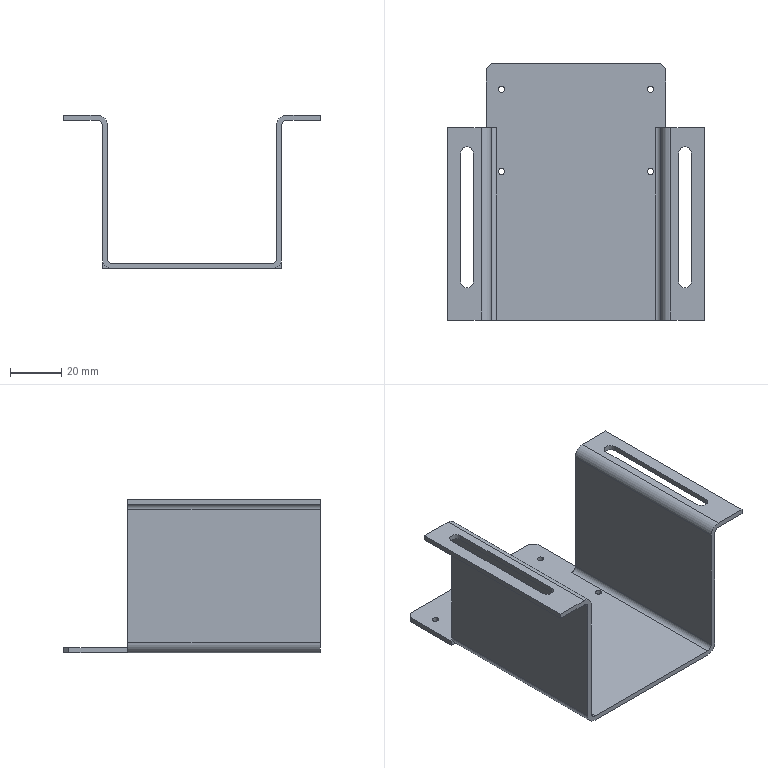Part | NX | features solid 2 | 1 solid | 48 faces | box 100 x 100 x 60 mm | volume 34001 mm3 | plane 28 | cylinder 20 | commonest cylinder face diameters 2.459 x8 4 x4 5 x4 8 x4
STEP:
#1=CARTESIAN_POINT('',(-907.77,471.,1235.));
#2=VERTEX_POINT('',#1);
#3=CARTESIAN_POINT('',(-907.77,471.,1237.));
#4=VERTEX_POINT('',#3);
#5=CARTESIAN_POINT('',(-907.77,471.,1388.623));
#6=DIRECTION('',(0.,0.,-1.));
#7=VECTOR('',#6,1000.);
#8=LINE('',#5,#7);
#9=EDGE_CURVE('',#2,#4,#8,.F.);
#10=ORIENTED_EDGE('',*,*,#9,.T.);
#11=CARTESIAN_POINT('',(-910.23,471.,1237.));
#12=VERTEX_POINT('',#11);
#13=CARTESIAN_POINT('',(-909.,471.,1237.));
#14=DIRECTION('',(0.,0.,-1.));
#15=DIRECTION('',(-1.,0.,0.));
#16=AXIS2_PLACEMENT_3D('',#13,#14,#15);
#17=CIRCLE('',#16,1.23);
#18=EDGE_CURVE('',#12,#4,#17,.T.);
#19=ORIENTED_EDGE('',*,*,#18,.F.);
#20=CARTESIAN_POINT('',(-910.23,471.,1235.));
#21=VERTEX_POINT('',#20);
#22=CARTESIAN_POINT('',(-910.23,471.,1388.623));
#23=DIRECTION('',(0.,0.,-1.));
#24=VECTOR('',#23,1000.);
#25=LINE('',#22,#24);
#26=EDGE_CURVE('',#12,#21,#25,.T.);
#27=ORIENTED_EDGE('',*,*,#26,.T.);
#28=CARTESIAN_POINT('',(-909.,471.,1235.));
#29=DIRECTION('',(0.,0.,-1.));
#30=DIRECTION('',(0.,1.,0.));
#31=AXIS2_PLACEMENT_3D('',#28,#29,#30);
#32=CIRCLE('',#31,1.23);
#33=EDGE_CURVE('',#21,#2,#32,.T.);
#34=ORIENTED_EDGE('',*,*,#33,.T.);
#35=EDGE_LOOP('',(#10,#19,#27,#34));
#36=FACE_BOUND('',#35,.T.);
#37=CARTESIAN_POINT('',(-909.,471.,1388.623));
#38=DIRECTION('',(0.,0.,-1.));
#39=DIRECTION('',(-1.,0.,0.));
#40=AXIS2_PLACEMENT_3D('',#37,#38,#39);
#41=CYLINDRICAL_SURFACE('',#40,1.23);
#42=ADVANCED_FACE('',(#36),#41,.F.);
#43=CARTESIAN_POINT('',(-965.77,471.,1237.));
#44=VERTEX_POINT('',#43);
#45=CARTESIAN_POINT('',(-965.77,471.,1235.));
#46=VERTEX_POINT('',#45);
#47=CARTESIAN_POINT('',(-965.77,471.,1388.623));
#48=DIRECTION('',(0.,0.,-1.));
#49=VECTOR('',#48,1000.);
#50=LINE('',#47,#49);
#51=EDGE_CURVE('',#44,#46,#50,.T.);
#52=ORIENTED_EDGE('',*,*,#51,.F.);
#53=CARTESIAN_POINT('',(-968.23,471.,1237.));
#54=VERTEX_POINT('',#53);
#55=CARTESIAN_POINT('',(-967.,471.,1237.));
#56=DIRECTION('',(0.,0.,-1.));
#57=DIRECTION('',(-1.,0.,0.));
#58=AXIS2_PLACEMENT_3D('',#55,#56,#57);
#59=CIRCLE('',#58,1.23);
#60=EDGE_CURVE('',#54,#44,#59,.T.);
#61=ORIENTED_EDGE('',*,*,#60,.F.);
#62=CARTESIAN_POINT('',(-968.23,471.,1235.));
#63=VERTEX_POINT('',#62);
#64=CARTESIAN_POINT('',(-968.23,471.,1388.623));
#65=DIRECTION('',(0.,0.,-1.));
#66=VECTOR('',#65,1000.);
#67=LINE('',#64,#66);
#68=EDGE_CURVE('',#63,#54,#67,.F.);
#69=ORIENTED_EDGE('',*,*,#68,.F.);
#70=CARTESIAN_POINT('',(-967.,471.,1235.));
#71=DIRECTION('',(0.,0.,-1.));
#72=DIRECTION('',(0.,1.,0.));
#73=AXIS2_PLACEMENT_3D('',#70,#71,#72);
#74=CIRCLE('',#73,1.23);
#75=EDGE_CURVE('',#63,#46,#74,.T.);
#76=ORIENTED_EDGE('',*,*,#75,.T.);
#77=EDGE_LOOP('',(#52,#61,#69,#76));
#78=FACE_BOUND('',#77,.T.);
#79=CARTESIAN_POINT('',(-967.,471.,1388.623));
#80=DIRECTION('',(0.,0.,-1.));
#81=DIRECTION('',(-1.,0.,0.));
#82=AXIS2_PLACEMENT_3D('',#79,#80,#81);
#83=CYLINDRICAL_SURFACE('',#82,1.23);
#84=ADVANCED_FACE('',(#78),#83,.F.);
#85=CARTESIAN_POINT('',(-965.77,503.,1235.));
#86=VERTEX_POINT('',#85);
#87=CARTESIAN_POINT('',(-965.77,503.,1237.));
#88=VERTEX_POINT('',#87);
#89=CARTESIAN_POINT('',(-965.77,503.,1388.623));
#90=DIRECTION('',(0.,0.,-1.));
#91=VECTOR('',#90,1000.);
#92=LINE('',#89,#91);
#93=EDGE_CURVE('',#86,#88,#92,.F.);
#94=ORIENTED_EDGE('',*,*,#93,.T.);
#95=CARTESIAN_POINT('',(-968.23,503.,1237.));
#96=VERTEX_POINT('',#95);
#97=CARTESIAN_POINT('',(-967.,503.,1237.));
#98=DIRECTION('',(0.,0.,-1.));
#99=DIRECTION('',(-1.,0.,0.));
#100=AXIS2_PLACEMENT_3D('',#97,#98,#99);
#101=CIRCLE('',#100,1.23);
#102=EDGE_CURVE('',#96,#88,#101,.T.);
#103=ORIENTED_EDGE('',*,*,#102,.F.);
#104=CARTESIAN_POINT('',(-968.23,503.,1235.));
#105=VERTEX_POINT('',#104);
#106=CARTESIAN_POINT('',(-968.23,503.,1388.623));
#107=DIRECTION('',(0.,0.,-1.));
#108=VECTOR('',#107,1000.);
#109=LINE('',#106,#108);
#110=EDGE_CURVE('',#96,#105,#109,.T.);
#111=ORIENTED_EDGE('',*,*,#110,.T.);
#112=CARTESIAN_POINT('',(-967.,503.,1235.));
#113=DIRECTION('',(0.,0.,-1.));
#114=DIRECTION('',(0.,1.,0.));
#115=AXIS2_PLACEMENT_3D('',#112,#113,#114);
#116=CIRCLE('',#115,1.23);
#117=EDGE_CURVE('',#105,#86,#116,.T.);
#118=ORIENTED_EDGE('',*,*,#117,.T.);
#119=EDGE_LOOP('',(#94,#103,#111,#118));
#120=FACE_BOUND('',#119,.T.);
#121=CARTESIAN_POINT('',(-967.,503.,1388.623));
#122=DIRECTION('',(0.,0.,-1.));
#123=DIRECTION('',(-1.,0.,0.));
#124=AXIS2_PLACEMENT_3D('',#121,#122,#123);
#125=CYLINDRICAL_SURFACE('',#124,1.23);
#126=ADVANCED_FACE('',(#120),#125,.F.);
#127=CARTESIAN_POINT('',(-907.77,503.,1235.));
#128=VERTEX_POINT('',#127);
#129=CARTESIAN_POINT('',(-907.77,503.,1237.));
#130=VERTEX_POINT('',#129);
#131=CARTESIAN_POINT('',(-907.77,503.,1388.623));
#132=DIRECTION('',(0.,0.,-1.));
#133=VECTOR('',#132,1000.);
#134=LINE('',#131,#133);
#135=EDGE_CURVE('',#128,#130,#134,.F.);
#136=ORIENTED_EDGE('',*,*,#135,.T.);
#137=CARTESIAN_POINT('',(-910.23,503.,1237.));
#138=VERTEX_POINT('',#137);
#139=CARTESIAN_POINT('',(-909.,503.,1237.));
#140=DIRECTION('',(0.,0.,-1.));
#141=DIRECTION('',(-1.,0.,0.));
#142=AXIS2_PLACEMENT_3D('',#139,#140,#141);
#143=CIRCLE('',#142,1.23);
#144=EDGE_CURVE('',#138,#130,#143,.T.);
#145=ORIENTED_EDGE('',*,*,#144,.F.);
#146=CARTESIAN_POINT('',(-910.23,503.,1235.));
#147=VERTEX_POINT('',#146);
#148=CARTESIAN_POINT('',(-910.23,503.,1388.623));
#149=DIRECTION('',(0.,0.,-1.));
#150=VECTOR('',#149,1000.);
#151=LINE('',#148,#150);
#152=EDGE_CURVE('',#138,#147,#151,.T.);
#153=ORIENTED_EDGE('',*,*,#152,.T.);
#154=CARTESIAN_POINT('',(-909.,503.,1235.));
#155=DIRECTION('',(0.,0.,-1.));
#156=DIRECTION('',(0.,1.,0.));
#157=AXIS2_PLACEMENT_3D('',#154,#155,#156);
#158=CIRCLE('',#157,1.23);
#159=EDGE_CURVE('',#147,#128,#158,.T.);
#160=ORIENTED_EDGE('',*,*,#159,.T.);
#161=EDGE_LOOP('',(#136,#145,#153,#160));
#162=FACE_BOUND('',#161,.T.);
#163=CARTESIAN_POINT('',(-909.,503.,1388.623));
#164=DIRECTION('',(0.,0.,-1.));
#165=DIRECTION('',(-1.,0.,0.));
#166=AXIS2_PLACEMENT_3D('',#163,#164,#165);
#167=CYLINDRICAL_SURFACE('',#166,1.23);
#168=ADVANCED_FACE('',(#162),#167,.F.);
#169=CARTESIAN_POINT('',(-978.,478.,1295.));
#170=VERTEX_POINT('',#169);
#171=CARTESIAN_POINT('',(-983.,478.,1295.));
#172=VERTEX_POINT('',#171);
#173=CARTESIAN_POINT('',(-980.5,478.,1295.));
#174=DIRECTION('',(0.,0.,1.));
#175=DIRECTION('',(1.,0.,0.));
#176=AXIS2_PLACEMENT_3D('',#173,#174,#175);
#177=CIRCLE('',#176,2.5);
#178=EDGE_CURVE('',#170,#172,#177,.T.);
#179=ORIENTED_EDGE('',*,*,#178,.T.);
#180=CARTESIAN_POINT('',(-983.,478.,1293.));
#181=VERTEX_POINT('',#180);
#182=CARTESIAN_POINT('',(-983.,478.,1321.));
#183=DIRECTION('',(0.,0.,-1.));
#184=VECTOR('',#183,1000.);
#185=LINE('',#182,#184);
#186=EDGE_CURVE('',#172,#181,#185,.T.);
#187=ORIENTED_EDGE('',*,*,#186,.T.);
#188=CARTESIAN_POINT('',(-978.,478.,1293.));
#189=VERTEX_POINT('',#188);
#190=CARTESIAN_POINT('',(-980.5,478.,1293.));
#191=DIRECTION('',(0.,0.,-1.));
#192=DIRECTION('',(0.,-1.,0.));
#193=AXIS2_PLACEMENT_3D('',#190,#191,#192);
#194=CIRCLE('',#193,2.5);
#195=EDGE_CURVE('',#181,#189,#194,.T.);
#196=ORIENTED_EDGE('',*,*,#195,.T.);
#197=CARTESIAN_POINT('',(-978.,478.,1321.));
#198=DIRECTION('',(0.,0.,-1.));
#199=VECTOR('',#198,1000.);
#200=LINE('',#197,#199);
#201=EDGE_CURVE('',#170,#189,#200,.T.);
#202=ORIENTED_EDGE('',*,*,#201,.F.);
#203=EDGE_LOOP('',(#179,#187,#196,#202));
#204=FACE_BOUND('',#203,.T.);
#205=CARTESIAN_POINT('',(-980.5,478.,1321.));
#206=DIRECTION('',(0.,0.,-1.));
#207=DIRECTION('',(-1.,0.,0.));
#208=AXIS2_PLACEMENT_3D('',#205,#206,#207);
#209=CYLINDRICAL_SURFACE('',#208,2.5);
#210=ADVANCED_FACE('',(#204),#209,.F.);
#211=CARTESIAN_POINT('',(-983.,428.,1295.));
#212=VERTEX_POINT('',#211);
#213=CARTESIAN_POINT('',(-983.,413.,1295.));
#214=DIRECTION('',(0.,-1.,0.));
#215=VECTOR('',#214,1000.);
#216=LINE('',#213,#215);
#217=EDGE_CURVE('',#172,#212,#216,.T.);
#218=ORIENTED_EDGE('',*,*,#217,.T.);
#219=CARTESIAN_POINT('',(-983.,428.,1293.));
#220=VERTEX_POINT('',#219);
#221=CARTESIAN_POINT('',(-983.,428.,1321.));
#222=DIRECTION('',(0.,0.,-1.));
#223=VECTOR('',#222,1000.);
#224=LINE('',#221,#223);
#225=EDGE_CURVE('',#212,#220,#224,.T.);
#226=ORIENTED_EDGE('',*,*,#225,.T.);
#227=CARTESIAN_POINT('',(-983.,428.,1293.));
#228=DIRECTION('',(0.,1.,0.));
#229=VECTOR('',#228,1000.);
#230=LINE('',#227,#229);
#231=EDGE_CURVE('',#220,#181,#230,.T.);
#232=ORIENTED_EDGE('',*,*,#231,.T.);
#233=ORIENTED_EDGE('',*,*,#186,.F.);
#234=EDGE_LOOP('',(#218,#226,#232,#233));
#235=FACE_BOUND('',#234,.T.);
#236=CARTESIAN_POINT('',(-983.,428.,1321.));
#237=DIRECTION('',(-1.,0.,0.));
#238=DIRECTION('',(0.,0.,1.));
#239=AXIS2_PLACEMENT_3D('',#236,#237,#238);
#240=PLANE('',#239);
#241=ADVANCED_FACE('',(#235),#240,.F.);
#242=CARTESIAN_POINT('',(-978.,428.,1295.));
#243=VERTEX_POINT('',#242);
#244=CARTESIAN_POINT('',(-980.5,428.,1295.));
#245=DIRECTION('',(0.,0.,1.));
#246=DIRECTION('',(1.,0.,0.));
#247=AXIS2_PLACEMENT_3D('',#244,#245,#246);
#248=CIRCLE('',#247,2.5);
#249=EDGE_CURVE('',#212,#243,#248,.T.);
#250=ORIENTED_EDGE('',*,*,#249,.T.);
#251=CARTESIAN_POINT('',(-978.,428.,1293.));
#252=VERTEX_POINT('',#251);
#253=CARTESIAN_POINT('',(-978.,428.,1321.));
#254=DIRECTION('',(0.,0.,-1.));
#255=VECTOR('',#254,1000.);
#256=LINE('',#253,#255);
#257=EDGE_CURVE('',#243,#252,#256,.T.);
#258=ORIENTED_EDGE('',*,*,#257,.T.);
#259=CARTESIAN_POINT('',(-980.5,428.,1293.));
#260=DIRECTION('',(0.,0.,-1.));
#261=DIRECTION('',(0.,1.,0.));
#262=AXIS2_PLACEMENT_3D('',#259,#260,#261);
#263=CIRCLE('',#262,2.5);
#264=EDGE_CURVE('',#252,#220,#263,.T.);
#265=ORIENTED_EDGE('',*,*,#264,.T.);
#266=ORIENTED_EDGE('',*,*,#225,.F.);
#267=EDGE_LOOP('',(#250,#258,#265,#266));
#268=FACE_BOUND('',#267,.T.);
#269=CARTESIAN_POINT('',(-980.5,428.,1321.));
#270=DIRECTION('',(0.,0.,-1.));
#271=DIRECTION('',(-1.,0.,0.));
#272=AXIS2_PLACEMENT_3D('',#269,#270,#271);
#273=CYLINDRICAL_SURFACE('',#272,2.5);
#274=ADVANCED_FACE('',(#268),#273,.F.);
#275=CARTESIAN_POINT('',(-978.,413.,1295.));
#276=DIRECTION('',(0.,1.,0.));
#277=VECTOR('',#276,1000.);
#278=LINE('',#275,#277);
#279=EDGE_CURVE('',#243,#170,#278,.T.);
#280=ORIENTED_EDGE('',*,*,#279,.T.);
#281=ORIENTED_EDGE('',*,*,#201,.T.);
#282=CARTESIAN_POINT('',(-978.,428.,1293.));
#283=DIRECTION('',(0.,-1.,0.));
#284=VECTOR('',#283,1000.);
#285=LINE('',#282,#284);
#286=EDGE_CURVE('',#189,#252,#285,.T.);
#287=ORIENTED_EDGE('',*,*,#286,.T.);
#288=ORIENTED_EDGE('',*,*,#257,.F.);
#289=EDGE_LOOP('',(#280,#281,#287,#288));
#290=FACE_BOUND('',#289,.T.);
#291=CARTESIAN_POINT('',(-978.,428.,1321.));
#292=DIRECTION('',(1.,0.,0.));
#293=DIRECTION('',(0.,0.,1.));
#294=AXIS2_PLACEMENT_3D('',#291,#292,#293);
#295=PLANE('',#294);
#296=ADVANCED_FACE('',(#290),#295,.F.);
#297=CARTESIAN_POINT('',(-893.,478.,1295.));
#298=VERTEX_POINT('',#297);
#299=CARTESIAN_POINT('',(-898.,478.,1295.));
#300=VERTEX_POINT('',#299);
#301=CARTESIAN_POINT('',(-895.5,478.,1295.));
#302=DIRECTION('',(0.,0.,1.));
#303=DIRECTION('',(1.,0.,0.));
#304=AXIS2_PLACEMENT_3D('',#301,#302,#303);
#305=CIRCLE('',#304,2.5);
#306=EDGE_CURVE('',#298,#300,#305,.T.);
#307=ORIENTED_EDGE('',*,*,#306,.T.);
#308=CARTESIAN_POINT('',(-898.,478.,1293.));
#309=VERTEX_POINT('',#308);
#310=CARTESIAN_POINT('',(-898.,478.,1321.));
#311=DIRECTION('',(0.,0.,-1.));
#312=VECTOR('',#311,1000.);
#313=LINE('',#310,#312);
#314=EDGE_CURVE('',#300,#309,#313,.T.);
#315=ORIENTED_EDGE('',*,*,#314,.T.);
#316=CARTESIAN_POINT('',(-893.,478.,1293.));
#317=VERTEX_POINT('',#316);
#318=CARTESIAN_POINT('',(-895.5,478.,1293.));
#319=DIRECTION('',(0.,0.,-1.));
#320=DIRECTION('',(0.,-1.,0.));
#321=AXIS2_PLACEMENT_3D('',#318,#319,#320);
#322=CIRCLE('',#321,2.5);
#323=EDGE_CURVE('',#309,#317,#322,.T.);
#324=ORIENTED_EDGE('',*,*,#323,.T.);
#325=CARTESIAN_POINT('',(-893.,478.,1321.));
#326=DIRECTION('',(0.,0.,-1.));
#327=VECTOR('',#326,1000.);
#328=LINE('',#325,#327);
#329=EDGE_CURVE('',#298,#317,#328,.T.);
#330=ORIENTED_EDGE('',*,*,#329,.F.);
#331=EDGE_LOOP('',(#307,#315,#324,#330));
#332=FACE_BOUND('',#331,.T.);
#333=CARTESIAN_POINT('',(-895.5,478.,1321.));
#334=DIRECTION('',(0.,0.,-1.));
#335=DIRECTION('',(-1.,0.,0.));
#336=AXIS2_PLACEMENT_3D('',#333,#334,#335);
#337=CYLINDRICAL_SURFACE('',#336,2.5);
#338=ADVANCED_FACE('',(#332),#337,.F.);
#339=CARTESIAN_POINT('',(-898.,428.,1295.));
#340=VERTEX_POINT('',#339);
#341=CARTESIAN_POINT('',(-898.,488.,1295.));
#342=DIRECTION('',(0.,-1.,0.));
#343=VECTOR('',#342,1000.);
#344=LINE('',#341,#343);
#345=EDGE_CURVE('',#300,#340,#344,.T.);
#346=ORIENTED_EDGE('',*,*,#345,.T.);
#347=CARTESIAN_POINT('',(-898.,428.,1293.));
#348=VERTEX_POINT('',#347);
#349=CARTESIAN_POINT('',(-898.,428.,1321.));
#350=DIRECTION('',(0.,0.,-1.));
#351=VECTOR('',#350,1000.);
#352=LINE('',#349,#351);
#353=EDGE_CURVE('',#340,#348,#352,.T.);
#354=ORIENTED_EDGE('',*,*,#353,.T.);
#355=CARTESIAN_POINT('',(-898.,428.,1293.));
#356=DIRECTION('',(0.,1.,0.));
#357=VECTOR('',#356,1000.);
#358=LINE('',#355,#357);
#359=EDGE_CURVE('',#348,#309,#358,.T.);
#360=ORIENTED_EDGE('',*,*,#359,.T.);
#361=ORIENTED_EDGE('',*,*,#314,.F.);
#362=EDGE_LOOP('',(#346,#354,#360,#361));
#363=FACE_BOUND('',#362,.T.);
#364=CARTESIAN_POINT('',(-898.,428.,1321.));
#365=DIRECTION('',(-1.,0.,0.));
#366=DIRECTION('',(0.,0.,1.));
#367=AXIS2_PLACEMENT_3D('',#364,#365,#366);
#368=PLANE('',#367);
#369=ADVANCED_FACE('',(#363),#368,.F.);
#370=CARTESIAN_POINT('',(-893.,428.,1295.));
#371=VERTEX_POINT('',#370);
#372=CARTESIAN_POINT('',(-895.5,428.,1295.));
#373=DIRECTION('',(0.,0.,1.));
#374=DIRECTION('',(1.,0.,0.));
#375=AXIS2_PLACEMENT_3D('',#372,#373,#374);
#376=CIRCLE('',#375,2.5);
#377=EDGE_CURVE('',#340,#371,#376,.T.);
#378=ORIENTED_EDGE('',*,*,#377,.T.);
#379=CARTESIAN_POINT('',(-893.,428.,1293.));
#380=VERTEX_POINT('',#379);
#381=CARTESIAN_POINT('',(-893.,428.,1321.));
#382=DIRECTION('',(0.,0.,-1.));
#383=VECTOR('',#382,1000.);
#384=LINE('',#381,#383);
#385=EDGE_CURVE('',#371,#380,#384,.T.);
#386=ORIENTED_EDGE('',*,*,#385,.T.);
#387=CARTESIAN_POINT('',(-895.5,428.,1293.));
#388=DIRECTION('',(0.,0.,-1.));
#389=DIRECTION('',(0.,1.,0.));
#390=AXIS2_PLACEMENT_3D('',#387,#388,#389);
#391=CIRCLE('',#390,2.5);
#392=EDGE_CURVE('',#380,#348,#391,.T.);
#393=ORIENTED_EDGE('',*,*,#392,.T.);
#394=ORIENTED_EDGE('',*,*,#353,.F.);
#395=EDGE_LOOP('',(#378,#386,#393,#394));
#396=FACE_BOUND('',#395,.T.);
#397=CARTESIAN_POINT('',(-895.5,428.,1321.));
#398=DIRECTION('',(0.,0.,-1.));
#399=DIRECTION('',(-1.,0.,0.));
#400=AXIS2_PLACEMENT_3D('',#397,#398,#399);
#401=CYLINDRICAL_SURFACE('',#400,2.5);
#402=ADVANCED_FACE('',(#396),#401,.F.);
#403=CARTESIAN_POINT('',(-893.,488.,1295.));
#404=DIRECTION('',(0.,1.,0.));
#405=VECTOR('',#404,1000.);
#406=LINE('',#403,#405);
#407=EDGE_CURVE('',#371,#298,#406,.T.);
#408=ORIENTED_EDGE('',*,*,#407,.T.);
#409=ORIENTED_EDGE('',*,*,#329,.T.);
#410=CARTESIAN_POINT('',(-893.,428.,1293.));
#411=DIRECTION('',(0.,-1.,0.));
#412=VECTOR('',#411,1000.);
#413=LINE('',#410,#412);
#414=EDGE_CURVE('',#317,#380,#413,.T.);
#415=ORIENTED_EDGE('',*,*,#414,.T.);
#416=ORIENTED_EDGE('',*,*,#385,.F.);
#417=EDGE_LOOP('',(#408,#409,#415,#416));
#418=FACE_BOUND('',#417,.T.);
#419=CARTESIAN_POINT('',(-893.,428.,1321.));
#420=DIRECTION('',(1.,0.,0.));
#421=DIRECTION('',(0.,0.,1.));
#422=AXIS2_PLACEMENT_3D('',#419,#420,#421);
#423=PLANE('',#422);
#424=ADVANCED_FACE('',(#418),#423,.F.);
#425=CARTESIAN_POINT('',(-905.,513.,1235.));
#426=VERTEX_POINT('',#425);
#427=CARTESIAN_POINT('',(-903.,511.,1235.));
#428=VERTEX_POINT('',#427);
#429=CARTESIAN_POINT('',(-854.,462.,1235.));
#430=DIRECTION('',(0.7071,-0.7071,0.));
#431=VECTOR('',#430,1000.);
#432=LINE('',#429,#431);
#433=EDGE_CURVE('',#426,#428,#432,.T.);
#434=ORIENTED_EDGE('',*,*,#433,.F.);
#435=CARTESIAN_POINT('',(-905.,513.,1237.));
#436=VERTEX_POINT('',#435);
#437=CARTESIAN_POINT('',(-905.,513.,1235.));
#438=DIRECTION('',(0.,0.,-1.));
#439=VECTOR('',#438,1000.);
#440=LINE('',#437,#439);
#441=EDGE_CURVE('',#436,#426,#440,.T.);
#442=ORIENTED_EDGE('',*,*,#441,.F.);
#443=CARTESIAN_POINT('',(-903.,511.,1237.));
#444=VERTEX_POINT('',#443);
#445=CARTESIAN_POINT('',(-903.,511.,1237.));
#446=DIRECTION('',(-0.7071,0.7071,0.));
#447=VECTOR('',#446,1000.);
#448=LINE('',#445,#447);
#449=EDGE_CURVE('',#444,#436,#448,.T.);
#450=ORIENTED_EDGE('',*,*,#449,.F.);
#451=CARTESIAN_POINT('',(-903.,511.,1235.));
#452=DIRECTION('',(0.,0.,1.));
#453=VECTOR('',#452,1000.);
#454=LINE('',#451,#453);
#455=EDGE_CURVE('',#428,#444,#454,.T.);
#456=ORIENTED_EDGE('',*,*,#455,.F.);
#457=EDGE_LOOP('',(#434,#442,#450,#456));
#458=FACE_BOUND('',#457,.T.);
#459=CARTESIAN_POINT('',(-903.,511.,1235.));
#460=DIRECTION('',(-0.7071,-0.7071,0.));
#461=DIRECTION('',(-0.7071,0.7071,0.));
#462=AXIS2_PLACEMENT_3D('',#459,#460,#461);
#463=PLANE('',#462);
#464=ADVANCED_FACE('',(#458),#463,.F.);
#465=CARTESIAN_POINT('',(-973.,511.,1235.));
#466=VERTEX_POINT('',#465);
#467=CARTESIAN_POINT('',(-971.,513.,1235.));
#468=VERTEX_POINT('',#467);
#469=CARTESIAN_POINT('',(-987.,497.,1235.));
#470=DIRECTION('',(0.7071,0.7071,0.));
#471=VECTOR('',#470,1000.);
#472=LINE('',#469,#471);
#473=EDGE_CURVE('',#466,#468,#472,.T.);
#474=ORIENTED_EDGE('',*,*,#473,.F.);
#475=CARTESIAN_POINT('',(-973.,511.,1237.));
#476=VERTEX_POINT('',#475);
#477=CARTESIAN_POINT('',(-973.,511.,1235.));
#478=DIRECTION('',(0.,0.,-1.));
#479=VECTOR('',#478,1000.);
#480=LINE('',#477,#479);
#481=EDGE_CURVE('',#476,#466,#480,.T.);
#482=ORIENTED_EDGE('',*,*,#481,.F.);
#483=CARTESIAN_POINT('',(-971.,513.,1237.));
#484=VERTEX_POINT('',#483);
#485=CARTESIAN_POINT('',(-971.,513.,1237.));
#486=DIRECTION('',(-0.7071,-0.7071,0.));
#487=VECTOR('',#486,1000.);
#488=LINE('',#485,#487);
#489=EDGE_CURVE('',#484,#476,#488,.T.);
#490=ORIENTED_EDGE('',*,*,#489,.F.);
#491=CARTESIAN_POINT('',(-971.,513.,1235.));
#492=DIRECTION('',(0.,0.,1.));
#493=VECTOR('',#492,1000.);
#494=LINE('',#491,#493);
#495=EDGE_CURVE('',#468,#484,#494,.T.);
#496=ORIENTED_EDGE('',*,*,#495,.F.);
#497=EDGE_LOOP('',(#474,#482,#490,#496));
#498=FACE_BOUND('',#497,.T.);
#499=CARTESIAN_POINT('',(-971.,513.,1235.));
#500=DIRECTION('',(0.7071,-0.7071,0.));
#501=DIRECTION('',(0.,0.,-1.));
#502=AXIS2_PLACEMENT_3D('',#499,#500,#501);
#503=PLANE('',#502);
#504=ADVANCED_FACE('',(#498),#503,.F.);
#505=CARTESIAN_POINT('',(-903.,413.,1291.));
#506=VERTEX_POINT('',#505);
#507=CARTESIAN_POINT('',(-903.,488.,1291.));
#508=VERTEX_POINT('',#507);
#509=CARTESIAN_POINT('',(-903.,413.,1291.));
#510=DIRECTION('',(0.,1.,0.));
#511=VECTOR('',#510,1000.);
#512=LINE('',#509,#511);
#513=EDGE_CURVE('',#506,#508,#512,.T.);
#514=ORIENTED_EDGE('',*,*,#513,.T.);
#515=CARTESIAN_POINT('',(-901.,488.,1293.));
#516=VERTEX_POINT('',#515);
#517=CARTESIAN_POINT('',(-901.,488.,1291.));
#518=DIRECTION('',(0.,1.,0.));
#519=DIRECTION('',(0.,0.,-1.));
#520=AXIS2_PLACEMENT_3D('',#517,#518,#519);
#521=CIRCLE('',#520,2.);
#522=EDGE_CURVE('',#508,#516,#521,.T.);
#523=ORIENTED_EDGE('',*,*,#522,.T.);
#524=CARTESIAN_POINT('',(-901.,413.,1293.));
#525=VERTEX_POINT('',#524);
#526=CARTESIAN_POINT('',(-901.,488.,1293.));
#527=DIRECTION('',(0.,-1.,0.));
#528=VECTOR('',#527,1000.);
#529=LINE('',#526,#528);
#530=EDGE_CURVE('',#516,#525,#529,.T.);
#531=ORIENTED_EDGE('',*,*,#530,.T.);
#532=CARTESIAN_POINT('',(-901.,413.,1291.));
#533=DIRECTION('',(0.,-1.,0.));
#534=DIRECTION('',(0.,0.,-1.));
#535=AXIS2_PLACEMENT_3D('',#532,#533,#534);
#536=CIRCLE('',#535,2.);
#537=EDGE_CURVE('',#525,#506,#536,.T.);
#538=ORIENTED_EDGE('',*,*,#537,.T.);
#539=EDGE_LOOP('',(#514,#523,#531,#538));
#540=FACE_BOUND('',#539,.T.);
#541=CARTESIAN_POINT('',(-901.,413.,1291.));
#542=DIRECTION('',(0.,1.,0.));
#543=DIRECTION('',(1.,0.,0.));
#544=AXIS2_PLACEMENT_3D('',#541,#542,#543);
#545=CYLINDRICAL_SURFACE('',#544,2.);
#546=ADVANCED_FACE('',(#540),#545,.F.);
#547=CARTESIAN_POINT('',(-905.,413.,1291.));
#548=VERTEX_POINT('',#547);
#549=CARTESIAN_POINT('',(-905.,488.,1291.));
#550=VERTEX_POINT('',#549);
#551=CARTESIAN_POINT('',(-905.,413.,1291.));
#552=DIRECTION('',(0.,1.,0.));
#553=VECTOR('',#552,1000.);
#554=LINE('',#551,#553);
#555=EDGE_CURVE('',#548,#550,#554,.T.);
#556=ORIENTED_EDGE('',*,*,#555,.F.);
#557=CARTESIAN_POINT('',(-901.,413.,1295.));
#558=VERTEX_POINT('',#557);
#559=CARTESIAN_POINT('',(-901.,413.,1291.));
#560=DIRECTION('',(0.,-1.,0.));
#561=DIRECTION('',(1.,0.,0.));
#562=AXIS2_PLACEMENT_3D('',#559,#560,#561);
#563=CIRCLE('',#562,4.);
#564=EDGE_CURVE('',#558,#548,#563,.T.);
#565=ORIENTED_EDGE('',*,*,#564,.F.);
#566=CARTESIAN_POINT('',(-901.,488.,1295.));
#567=VERTEX_POINT('',#566);
#568=CARTESIAN_POINT('',(-901.,488.,1295.));
#569=DIRECTION('',(0.,-1.,0.));
#570=VECTOR('',#569,1000.);
#571=LINE('',#568,#570);
#572=EDGE_CURVE('',#567,#558,#571,.T.);
#573=ORIENTED_EDGE('',*,*,#572,.F.);
#574=CARTESIAN_POINT('',(-901.,488.,1291.));
#575=DIRECTION('',(0.,1.,0.));
#576=DIRECTION('',(1.,0.,0.));
#577=AXIS2_PLACEMENT_3D('',#574,#575,#576);
#578=CIRCLE('',#577,4.);
#579=EDGE_CURVE('',#550,#567,#578,.T.);
#580=ORIENTED_EDGE('',*,*,#579,.F.);
#581=EDGE_LOOP('',(#556,#565,#573,#580));
#582=FACE_BOUND('',#581,.T.);
#583=CARTESIAN_POINT('',(-901.,413.,1291.));
#584=DIRECTION('',(0.,1.,0.));
#585=DIRECTION('',(1.,0.,0.));
#586=AXIS2_PLACEMENT_3D('',#583,#584,#585);
#587=CYLINDRICAL_SURFACE('',#586,4.);
#588=ADVANCED_FACE('',(#582),#587,.T.);
#589=CARTESIAN_POINT('',(-888.,413.,1293.));
#590=VERTEX_POINT('',#589);
#591=CARTESIAN_POINT('',(-888.,488.,1293.));
#592=VERTEX_POINT('',#591);
#593=CARTESIAN_POINT('',(-888.,413.,1293.));
#594=DIRECTION('',(0.,1.,0.));
#595=VECTOR('',#594,1000.);
#596=LINE('',#593,#595);
#597=EDGE_CURVE('',#590,#592,#596,.T.);
#598=ORIENTED_EDGE('',*,*,#597,.T.);
#599=CARTESIAN_POINT('',(-888.,488.,1295.));
#600=VERTEX_POINT('',#599);
#601=CARTESIAN_POINT('',(-888.,488.,1295.));
#602=DIRECTION('',(0.,0.,-1.));
#603=VECTOR('',#602,1000.);
#604=LINE('',#601,#603);
#605=EDGE_CURVE('',#600,#592,#604,.T.);
#606=ORIENTED_EDGE('',*,*,#605,.F.);
#607=CARTESIAN_POINT('',(-888.,413.,1295.));
#608=VERTEX_POINT('',#607);
#609=CARTESIAN_POINT('',(-888.,413.,1295.));
#610=DIRECTION('',(0.,1.,0.));
#611=VECTOR('',#610,1000.);
#612=LINE('',#609,#611);
#613=EDGE_CURVE('',#608,#600,#612,.T.);
#614=ORIENTED_EDGE('',*,*,#613,.F.);
#615=CARTESIAN_POINT('',(-888.,413.,1295.));
#616=DIRECTION('',(0.,0.,-1.));
#617=VECTOR('',#616,1000.);
#618=LINE('',#615,#617);
#619=EDGE_CURVE('',#608,#590,#618,.T.);
#620=ORIENTED_EDGE('',*,*,#619,.T.);
#621=EDGE_LOOP('',(#598,#606,#614,#620));
#622=FACE_BOUND('',#621,.T.);
#623=CARTESIAN_POINT('',(-888.,413.,1295.));
#624=DIRECTION('',(-1.,0.,0.));
#625=DIRECTION('',(0.,0.,1.));
#626=AXIS2_PLACEMENT_3D('',#623,#624,#625);
#627=PLANE('',#626);
#628=ADVANCED_FACE('',(#622),#627,.F.);
#629=ORIENTED_EDGE('',*,*,#392,.F.);
#630=ORIENTED_EDGE('',*,*,#414,.F.);
#631=ORIENTED_EDGE('',*,*,#323,.F.);
#632=ORIENTED_EDGE('',*,*,#359,.F.);
#633=EDGE_LOOP('',(#629,#630,#631,#632));
#634=FACE_BOUND('',#633,.T.);
#635=ORIENTED_EDGE('',*,*,#530,.F.);
#636=CARTESIAN_POINT('',(-903.278,488.,1293.));
#637=DIRECTION('',(-1.,0.,0.));
#638=VECTOR('',#637,1000.);
#639=LINE('',#636,#638);
#640=EDGE_CURVE('',#592,#516,#639,.T.);
#641=ORIENTED_EDGE('',*,*,#640,.F.);
#642=ORIENTED_EDGE('',*,*,#597,.F.);
#643=CARTESIAN_POINT('',(-903.278,413.,1293.));
#644=DIRECTION('',(1.,0.,0.));
#645=VECTOR('',#644,1000.);
#646=LINE('',#643,#645);
#647=EDGE_CURVE('',#525,#590,#646,.T.);
#648=ORIENTED_EDGE('',*,*,#647,.F.);
#649=EDGE_LOOP('',(#635,#641,#642,#648));
#650=FACE_BOUND('',#649,.T.);
#651=CARTESIAN_POINT('',(-903.278,488.,1293.));
#652=DIRECTION('',(0.,0.,1.));
#653=DIRECTION('',(1.,0.,0.));
#654=AXIS2_PLACEMENT_3D('',#651,#652,#653);
#655=PLANE('',#654);
#656=ADVANCED_FACE('',(#634,#650),#655,.F.);
#657=ORIENTED_EDGE('',*,*,#407,.F.);
#658=ORIENTED_EDGE('',*,*,#377,.F.);
#659=ORIENTED_EDGE('',*,*,#345,.F.);
#660=ORIENTED_EDGE('',*,*,#306,.F.);
#661=EDGE_LOOP('',(#657,#658,#659,#660));
#662=FACE_BOUND('',#661,.T.);
#663=CARTESIAN_POINT('',(-903.278,488.,1295.));
#664=DIRECTION('',(-1.,0.,0.));
#665=VECTOR('',#664,1000.);
#666=LINE('',#663,#665);
#667=EDGE_CURVE('',#600,#567,#666,.T.);
#668=ORIENTED_EDGE('',*,*,#667,.T.);
#669=ORIENTED_EDGE('',*,*,#572,.T.);
#670=CARTESIAN_POINT('',(-903.278,413.,1295.));
#671=DIRECTION('',(1.,0.,0.));
#672=VECTOR('',#671,1000.);
#673=LINE('',#670,#672);
#674=EDGE_CURVE('',#558,#608,#673,.T.);
#675=ORIENTED_EDGE('',*,*,#674,.T.);
#676=ORIENTED_EDGE('',*,*,#613,.T.);
#677=EDGE_LOOP('',(#668,#669,#675,#676));
#678=FACE_BOUND('',#677,.T.);
#679=CARTESIAN_POINT('',(-903.278,488.,1295.));
#680=DIRECTION('',(0.,0.,1.));
#681=DIRECTION('',(1.,0.,0.));
#682=AXIS2_PLACEMENT_3D('',#679,#680,#681);
#683=PLANE('',#682);
#684=ADVANCED_FACE('',(#662,#678),#683,.T.);
#685=CARTESIAN_POINT('',(-973.,488.,1291.));
#686=VERTEX_POINT('',#685);
#687=CARTESIAN_POINT('',(-973.,413.,1291.));
#688=VERTEX_POINT('',#687);
#689=CARTESIAN_POINT('',(-973.,488.,1291.));
#690=DIRECTION('',(0.,-1.,0.));
#691=VECTOR('',#690,1000.);
#692=LINE('',#689,#691);
#693=EDGE_CURVE('',#686,#688,#692,.T.);
#694=ORIENTED_EDGE('',*,*,#693,.T.);
#695=CARTESIAN_POINT('',(-975.,413.,1293.));
#696=VERTEX_POINT('',#695);
#697=CARTESIAN_POINT('',(-975.,413.,1291.));
#698=DIRECTION('',(0.,-1.,0.));
#699=DIRECTION('',(0.,0.,1.));
#700=AXIS2_PLACEMENT_3D('',#697,#698,#699);
#701=CIRCLE('',#700,2.);
#702=EDGE_CURVE('',#688,#696,#701,.T.);
#703=ORIENTED_EDGE('',*,*,#702,.T.);
#704=CARTESIAN_POINT('',(-975.,488.,1293.));
#705=VERTEX_POINT('',#704);
#706=CARTESIAN_POINT('',(-975.,413.,1293.));
#707=DIRECTION('',(0.,1.,0.));
#708=VECTOR('',#707,1000.);
#709=LINE('',#706,#708);
#710=EDGE_CURVE('',#696,#705,#709,.T.);
#711=ORIENTED_EDGE('',*,*,#710,.T.);
#712=CARTESIAN_POINT('',(-975.,488.,1291.));
#713=DIRECTION('',(0.,1.,0.));
#714=DIRECTION('',(0.,0.,1.));
#715=AXIS2_PLACEMENT_3D('',#712,#713,#714);
#716=CIRCLE('',#715,2.);
#717=EDGE_CURVE('',#705,#686,#716,.T.);
#718=ORIENTED_EDGE('',*,*,#717,.T.);
#719=EDGE_LOOP('',(#694,#703,#711,#718));
#720=FACE_BOUND('',#719,.T.);
#721=CARTESIAN_POINT('',(-975.,488.,1291.));
#722=DIRECTION('',(0.,-1.,0.));
#723=DIRECTION('',(-1.,0.,0.));
#724=AXIS2_PLACEMENT_3D('',#721,#722,#723);
#725=CYLINDRICAL_SURFACE('',#724,2.);
#726=ADVANCED_FACE('',(#720),#725,.F.);
#727=CARTESIAN_POINT('',(-971.,488.,1291.));
#728=VERTEX_POINT('',#727);
#729=CARTESIAN_POINT('',(-971.,413.,1291.));
#730=VERTEX_POINT('',#729);
#731=CARTESIAN_POINT('',(-971.,488.,1291.));
#732=DIRECTION('',(0.,-1.,0.));
#733=VECTOR('',#732,1000.);
#734=LINE('',#731,#733);
#735=EDGE_CURVE('',#728,#730,#734,.T.);
#736=ORIENTED_EDGE('',*,*,#735,.F.);
#737=CARTESIAN_POINT('',(-975.,488.,1295.));
#738=VERTEX_POINT('',#737);
#739=CARTESIAN_POINT('',(-975.,488.,1291.));
#740=DIRECTION('',(0.,1.,0.));
#741=DIRECTION('',(-1.,0.,0.));
#742=AXIS2_PLACEMENT_3D('',#739,#740,#741);
#743=CIRCLE('',#742,4.);
#744=EDGE_CURVE('',#738,#728,#743,.T.);
#745=ORIENTED_EDGE('',*,*,#744,.F.);
#746=CARTESIAN_POINT('',(-975.,413.,1295.));
#747=VERTEX_POINT('',#746);
#748=CARTESIAN_POINT('',(-975.,413.,1295.));
#749=DIRECTION('',(0.,1.,0.));
#750=VECTOR('',#749,1000.);
#751=LINE('',#748,#750);
#752=EDGE_CURVE('',#747,#738,#751,.T.);
#753=ORIENTED_EDGE('',*,*,#752,.F.);
#754=CARTESIAN_POINT('',(-975.,413.,1291.));
#755=DIRECTION('',(0.,-1.,0.));
#756=DIRECTION('',(-1.,0.,0.));
#757=AXIS2_PLACEMENT_3D('',#754,#755,#756);
#758=CIRCLE('',#757,4.);
#759=EDGE_CURVE('',#730,#747,#758,.T.);
#760=ORIENTED_EDGE('',*,*,#759,.F.);
#761=EDGE_LOOP('',(#736,#745,#753,#760));
#762=FACE_BOUND('',#761,.T.);
#763=CARTESIAN_POINT('',(-975.,488.,1291.));
#764=DIRECTION('',(0.,-1.,0.));
#765=DIRECTION('',(-1.,0.,0.));
#766=AXIS2_PLACEMENT_3D('',#763,#764,#765);
#767=CYLINDRICAL_SURFACE('',#766,4.);
#768=ADVANCED_FACE('',(#762),#767,.T.);
#769=CARTESIAN_POINT('',(-988.,488.,1293.));
#770=VERTEX_POINT('',#769);
#771=CARTESIAN_POINT('',(-988.,413.,1293.));
#772=VERTEX_POINT('',#771);
#773=CARTESIAN_POINT('',(-988.,488.,1293.));
#774=DIRECTION('',(0.,-1.,0.));
#775=VECTOR('',#774,1000.);
#776=LINE('',#773,#775);
#777=EDGE_CURVE('',#770,#772,#776,.T.);
#778=ORIENTED_EDGE('',*,*,#777,.T.);
#779=CARTESIAN_POINT('',(-988.,413.,1295.));
#780=VERTEX_POINT('',#779);
#781=CARTESIAN_POINT('',(-988.,413.,1295.));
#782=DIRECTION('',(0.,0.,-1.));
#783=VECTOR('',#782,1000.);
#784=LINE('',#781,#783);
#785=EDGE_CURVE('',#780,#772,#784,.T.);
#786=ORIENTED_EDGE('',*,*,#785,.F.);
#787=CARTESIAN_POINT('',(-988.,488.,1295.));
#788=VERTEX_POINT('',#787);
#789=CARTESIAN_POINT('',(-988.,488.,1295.));
#790=DIRECTION('',(0.,-1.,0.));
#791=VECTOR('',#790,1000.);
#792=LINE('',#789,#791);
#793=EDGE_CURVE('',#788,#780,#792,.T.);
#794=ORIENTED_EDGE('',*,*,#793,.F.);
#795=CARTESIAN_POINT('',(-988.,488.,1295.));
#796=DIRECTION('',(0.,0.,-1.));
#797=VECTOR('',#796,1000.);
#798=LINE('',#795,#797);
#799=EDGE_CURVE('',#788,#770,#798,.T.);
#800=ORIENTED_EDGE('',*,*,#799,.T.);
#801=EDGE_LOOP('',(#778,#786,#794,#800));
#802=FACE_BOUND('',#801,.T.);
#803=CARTESIAN_POINT('',(-988.,488.,1295.));
#804=DIRECTION('',(1.,0.,0.));
#805=DIRECTION('',(0.,0.,1.));
#806=AXIS2_PLACEMENT_3D('',#803,#804,#805);
#807=PLANE('',#806);
#808=ADVANCED_FACE('',(#802),#807,.F.);
#809=ORIENTED_EDGE('',*,*,#264,.F.);
#810=ORIENTED_EDGE('',*,*,#286,.F.);
#811=ORIENTED_EDGE('',*,*,#195,.F.);
#812=ORIENTED_EDGE('',*,*,#231,.F.);
#813=EDGE_LOOP('',(#809,#810,#811,#812));
#814=FACE_BOUND('',#813,.T.);
#815=ORIENTED_EDGE('',*,*,#710,.F.);
#816=CARTESIAN_POINT('',(-972.722,413.,1293.));
#817=DIRECTION('',(1.,0.,0.));
#818=VECTOR('',#817,1000.);
#819=LINE('',#816,#818);
#820=EDGE_CURVE('',#772,#696,#819,.T.);
#821=ORIENTED_EDGE('',*,*,#820,.F.);
#822=ORIENTED_EDGE('',*,*,#777,.F.);
#823=CARTESIAN_POINT('',(-972.722,488.,1293.));
#824=DIRECTION('',(-1.,0.,0.));
#825=VECTOR('',#824,1000.);
#826=LINE('',#823,#825);
#827=EDGE_CURVE('',#705,#770,#826,.T.);
#828=ORIENTED_EDGE('',*,*,#827,.F.);
#829=EDGE_LOOP('',(#815,#821,#822,#828));
#830=FACE_BOUND('',#829,.T.);
#831=CARTESIAN_POINT('',(-972.722,413.,1293.));
#832=DIRECTION('',(0.,0.,1.));
#833=DIRECTION('',(1.,0.,0.));
#834=AXIS2_PLACEMENT_3D('',#831,#832,#833);
#835=PLANE('',#834);
#836=ADVANCED_FACE('',(#814,#830),#835,.F.);
#837=ORIENTED_EDGE('',*,*,#279,.F.);
#838=ORIENTED_EDGE('',*,*,#249,.F.);
#839=ORIENTED_EDGE('',*,*,#217,.F.);
#840=ORIENTED_EDGE('',*,*,#178,.F.);
#841=EDGE_LOOP('',(#837,#838,#839,#840));
#842=FACE_BOUND('',#841,.T.);
#843=CARTESIAN_POINT('',(-972.722,413.,1295.));
#844=DIRECTION('',(1.,0.,0.));
#845=VECTOR('',#844,1000.);
#846=LINE('',#843,#845);
#847=EDGE_CURVE('',#780,#747,#846,.T.);
#848=ORIENTED_EDGE('',*,*,#847,.T.);
#849=ORIENTED_EDGE('',*,*,#752,.T.);
#850=CARTESIAN_POINT('',(-972.722,488.,1295.));
#851=DIRECTION('',(-1.,0.,0.));
#852=VECTOR('',#851,1000.);
#853=LINE('',#850,#852);
#854=EDGE_CURVE('',#738,#788,#853,.T.);
#855=ORIENTED_EDGE('',*,*,#854,.T.);
#856=ORIENTED_EDGE('',*,*,#793,.T.);
#857=EDGE_LOOP('',(#848,#849,#855,#856));
#858=FACE_BOUND('',#857,.T.);
#859=CARTESIAN_POINT('',(-972.722,413.,1295.));
#860=DIRECTION('',(0.,0.,1.));
#861=DIRECTION('',(1.,0.,0.));
#862=AXIS2_PLACEMENT_3D('',#859,#860,#861);
#863=PLANE('',#862);
#864=ADVANCED_FACE('',(#842,#858),#863,.T.);
#865=CARTESIAN_POINT('',(-907.,488.,1237.));
#866=VERTEX_POINT('',#865);
#867=CARTESIAN_POINT('',(-907.,413.,1237.));
#868=VERTEX_POINT('',#867);
#869=CARTESIAN_POINT('',(-907.,488.,1237.));
#870=DIRECTION('',(0.,-1.,0.));
#871=VECTOR('',#870,1000.);
#872=LINE('',#869,#871);
#873=EDGE_CURVE('',#866,#868,#872,.T.);
#874=ORIENTED_EDGE('',*,*,#873,.T.);
#875=CARTESIAN_POINT('',(-905.,413.,1239.));
#876=VERTEX_POINT('',#875);
#877=CARTESIAN_POINT('',(-907.,413.,1239.));
#878=DIRECTION('',(0.,-1.,0.));
#879=DIRECTION('',(-1.,0.,0.));
#880=AXIS2_PLACEMENT_3D('',#877,#878,#879);
#881=CIRCLE('',#880,2.);
#882=EDGE_CURVE('',#868,#876,#881,.T.);
#883=ORIENTED_EDGE('',*,*,#882,.T.);
#884=CARTESIAN_POINT('',(-905.,488.,1239.));
#885=VERTEX_POINT('',#884);
#886=CARTESIAN_POINT('',(-905.,413.,1239.));
#887=DIRECTION('',(0.,1.,0.));
#888=VECTOR('',#887,1000.);
#889=LINE('',#886,#888);
#890=EDGE_CURVE('',#876,#885,#889,.T.);
#891=ORIENTED_EDGE('',*,*,#890,.T.);
#892=CARTESIAN_POINT('',(-907.,488.,1239.));
#893=DIRECTION('',(0.,1.,0.));
#894=DIRECTION('',(-1.,0.,0.));
#895=AXIS2_PLACEMENT_3D('',#892,#893,#894);
#896=CIRCLE('',#895,2.);
#897=EDGE_CURVE('',#885,#866,#896,.T.);
#898=ORIENTED_EDGE('',*,*,#897,.T.);
#899=EDGE_LOOP('',(#874,#883,#891,#898));
#900=FACE_BOUND('',#899,.T.);
#901=CARTESIAN_POINT('',(-907.,488.,1239.));
#902=DIRECTION('',(0.,-1.,0.));
#903=DIRECTION('',(0.,0.,1.));
#904=AXIS2_PLACEMENT_3D('',#901,#902,#903);
#905=CYLINDRICAL_SURFACE('',#904,2.);
#906=ADVANCED_FACE('',(#900),#905,.F.);
#907=CARTESIAN_POINT('',(-907.,488.,1235.));
#908=VERTEX_POINT('',#907);
#909=CARTESIAN_POINT('',(-907.,413.,1235.));
#910=VERTEX_POINT('',#909);
#911=CARTESIAN_POINT('',(-907.,488.,1235.));
#912=DIRECTION('',(0.,-1.,0.));
#913=VECTOR('',#912,1000.);
#914=LINE('',#911,#913);
#915=EDGE_CURVE('',#908,#910,#914,.T.);
#916=ORIENTED_EDGE('',*,*,#915,.F.);
#917=CARTESIAN_POINT('',(-903.,488.,1239.));
#918=VERTEX_POINT('',#917);
#919=CARTESIAN_POINT('',(-907.,488.,1239.));
#920=DIRECTION('',(0.,1.,0.));
#921=DIRECTION('',(0.,0.,1.));
#922=AXIS2_PLACEMENT_3D('',#919,#920,#921);
#923=CIRCLE('',#922,4.);
#924=EDGE_CURVE('',#918,#908,#923,.T.);
#925=ORIENTED_EDGE('',*,*,#924,.F.);
#926=CARTESIAN_POINT('',(-903.,413.,1239.));
#927=VERTEX_POINT('',#926);
#928=CARTESIAN_POINT('',(-903.,413.,1239.));
#929=DIRECTION('',(0.,1.,0.));
#930=VECTOR('',#929,1000.);
#931=LINE('',#928,#930);
#932=EDGE_CURVE('',#927,#918,#931,.T.);
#933=ORIENTED_EDGE('',*,*,#932,.F.);
#934=CARTESIAN_POINT('',(-907.,413.,1239.));
#935=DIRECTION('',(0.,-1.,0.));
#936=DIRECTION('',(0.,0.,1.));
#937=AXIS2_PLACEMENT_3D('',#934,#935,#936);
#938=CIRCLE('',#937,4.);
#939=EDGE_CURVE('',#910,#927,#938,.T.);
#940=ORIENTED_EDGE('',*,*,#939,.F.);
#941=EDGE_LOOP('',(#916,#925,#933,#940));
#942=FACE_BOUND('',#941,.T.);
#943=CARTESIAN_POINT('',(-907.,488.,1239.));
#944=DIRECTION('',(0.,-1.,0.));
#945=DIRECTION('',(0.,0.,1.));
#946=AXIS2_PLACEMENT_3D('',#943,#944,#945);
#947=CYLINDRICAL_SURFACE('',#946,4.);
#948=ADVANCED_FACE('',(#942),#947,.T.);
#949=ORIENTED_EDGE('',*,*,#513,.F.);
#950=CARTESIAN_POINT('',(-903.,413.,1236.722));
#951=DIRECTION('',(0.,0.,-1.));
#952=VECTOR('',#951,1000.);
#953=LINE('',#950,#952);
#954=EDGE_CURVE('',#506,#927,#953,.T.);
#955=ORIENTED_EDGE('',*,*,#954,.T.);
#956=ORIENTED_EDGE('',*,*,#932,.T.);
#957=CARTESIAN_POINT('',(-903.,488.,1236.722));
#958=DIRECTION('',(0.,0.,1.));
#959=VECTOR('',#958,1000.);
#960=LINE('',#957,#959);
#961=EDGE_CURVE('',#918,#508,#960,.T.);
#962=ORIENTED_EDGE('',*,*,#961,.T.);
#963=EDGE_LOOP('',(#949,#955,#956,#962));
#964=FACE_BOUND('',#963,.T.);
#965=CARTESIAN_POINT('',(-903.,413.,1236.722));
#966=DIRECTION('',(1.,0.,0.));
#967=DIRECTION('',(0.,0.,1.));
#968=AXIS2_PLACEMENT_3D('',#965,#966,#967);
#969=PLANE('',#968);
#970=ADVANCED_FACE('',(#964),#969,.T.);
#971=CARTESIAN_POINT('',(-907.1,488.,1237.));
#972=VERTEX_POINT('',#971);
#973=CARTESIAN_POINT('',(-907.1,488.1,1237.));
#974=VERTEX_POINT('',#973);
#975=CARTESIAN_POINT('',(-907.1,488.,1237.));
#976=DIRECTION('',(0.,1.,0.));
#977=VECTOR('',#976,1000.);
#978=LINE('',#975,#977);
#979=EDGE_CURVE('',#972,#974,#978,.T.);
#980=ORIENTED_EDGE('',*,*,#979,.F.);
#981=CARTESIAN_POINT('',(-907.1,488.,1235.));
#982=VERTEX_POINT('',#981);
#983=CARTESIAN_POINT('',(-907.1,488.,1235.));
#984=DIRECTION('',(0.,0.,-1.));
#985=VECTOR('',#984,1000.);
#986=LINE('',#983,#985);
#987=EDGE_CURVE('',#972,#982,#986,.T.);
#988=ORIENTED_EDGE('',*,*,#987,.T.);
#989=CARTESIAN_POINT('',(-907.1,488.1,1235.));
#990=VERTEX_POINT('',#989);
#991=CARTESIAN_POINT('',(-907.1,488.1,1235.));
#992=DIRECTION('',(0.,1.,0.));
#993=VECTOR('',#992,1000.);
#994=LINE('',#991,#993);
#995=EDGE_CURVE('',#982,#990,#994,.T.);
#996=ORIENTED_EDGE('',*,*,#995,.T.);
#997=CARTESIAN_POINT('',(-907.1,488.1,1235.));
#998=DIRECTION('',(0.,0.,-1.));
#999=VECTOR('',#998,1000.);
#1000=LINE('',#997,#999);
#1001=EDGE_CURVE('',#974,#990,#1000,.T.);
#1002=ORIENTED_EDGE('',*,*,#1001,.F.);
#1003=EDGE_LOOP('',(#980,#988,#996,#1002));
#1004=FACE_BOUND('',#1003,.T.);
#1005=CARTESIAN_POINT('',(-907.1,488.1,1235.));
#1006=DIRECTION('',(-1.,0.,0.));
#1007=DIRECTION('',(0.,0.,1.));
#1008=AXIS2_PLACEMENT_3D('',#1005,#1006,#1007);
#1009=PLANE('',#1008);
#1010=ADVANCED_FACE('',(#1004),#1009,.F.);
#1011=ORIENTED_EDGE('',*,*,#1001,.T.);
#1012=CARTESIAN_POINT('',(-903.,488.1,1235.));
#1013=VERTEX_POINT('',#1012);
#1014=CARTESIAN_POINT('',(-903.,488.1,1235.));
#1015=DIRECTION('',(1.,0.,0.));
#1016=VECTOR('',#1015,1000.);
#1017=LINE('',#1014,#1016);
#1018=EDGE_CURVE('',#990,#1013,#1017,.T.);
#1019=ORIENTED_EDGE('',*,*,#1018,.T.);
#1020=CARTESIAN_POINT('',(-903.,488.1,1237.));
#1021=VERTEX_POINT('',#1020);
#1022=CARTESIAN_POINT('',(-903.,488.1,1235.));
#1023=DIRECTION('',(0.,0.,-1.));
#1024=VECTOR('',#1023,1000.);
#1025=LINE('',#1022,#1024);
#1026=EDGE_CURVE('',#1021,#1013,#1025,.T.);
#1027=ORIENTED_EDGE('',*,*,#1026,.F.);
#1028=CARTESIAN_POINT('',(-907.1,488.1,1237.));
#1029=DIRECTION('',(1.,0.,0.));
#1030=VECTOR('',#1029,1000.);
#1031=LINE('',#1028,#1030);
#1032=EDGE_CURVE('',#974,#1021,#1031,.T.);
#1033=ORIENTED_EDGE('',*,*,#1032,.F.);
#1034=EDGE_LOOP('',(#1011,#1019,#1027,#1033));
#1035=FACE_BOUND('',#1034,.T.);
#1036=CARTESIAN_POINT('',(-903.,488.1,1235.));
#1037=DIRECTION('',(0.,1.,0.));
#1038=DIRECTION('',(1.,0.,0.));
#1039=AXIS2_PLACEMENT_3D('',#1036,#1037,#1038);
#1040=PLANE('',#1039);
#1041=ADVANCED_FACE('',(#1035),#1040,.F.);
#1042=CARTESIAN_POINT('',(-969.,413.,1237.));
#1043=VERTEX_POINT('',#1042);
#1044=CARTESIAN_POINT('',(-969.,488.,1237.));
#1045=VERTEX_POINT('',#1044);
#1046=CARTESIAN_POINT('',(-969.,413.,1237.));
#1047=DIRECTION('',(0.,1.,0.));
#1048=VECTOR('',#1047,1000.);
#1049=LINE('',#1046,#1048);
#1050=EDGE_CURVE('',#1043,#1045,#1049,.T.);
#1051=ORIENTED_EDGE('',*,*,#1050,.T.);
#1052=CARTESIAN_POINT('',(-971.,488.,1239.));
#1053=VERTEX_POINT('',#1052);
#1054=CARTESIAN_POINT('',(-969.,488.,1239.));
#1055=DIRECTION('',(0.,-1.,0.));
#1056=DIRECTION('',(1.,0.,0.));
#1057=AXIS2_PLACEMENT_3D('',#1054,#1055,#1056);
#1058=CIRCLE('',#1057,2.);
#1059=EDGE_CURVE('',#1053,#1045,#1058,.T.);
#1060=ORIENTED_EDGE('',*,*,#1059,.F.);
#1061=CARTESIAN_POINT('',(-971.,413.,1239.));
#1062=VERTEX_POINT('',#1061);
#1063=CARTESIAN_POINT('',(-971.,488.,1239.));
#1064=DIRECTION('',(0.,-1.,0.));
#1065=VECTOR('',#1064,1000.);
#1066=LINE('',#1063,#1065);
#1067=EDGE_CURVE('',#1053,#1062,#1066,.T.);
#1068=ORIENTED_EDGE('',*,*,#1067,.T.);
#1069=CARTESIAN_POINT('',(-969.,413.,1239.));
#1070=DIRECTION('',(0.,1.,0.));
#1071=DIRECTION('',(1.,0.,0.));
#1072=AXIS2_PLACEMENT_3D('',#1069,#1070,#1071);
#1073=CIRCLE('',#1072,2.);
#1074=EDGE_CURVE('',#1043,#1062,#1073,.T.);
#1075=ORIENTED_EDGE('',*,*,#1074,.F.);
#1076=EDGE_LOOP('',(#1051,#1060,#1068,#1075));
#1077=FACE_BOUND('',#1076,.T.);
#1078=CARTESIAN_POINT('',(-969.,413.,1239.));
#1079=DIRECTION('',(0.,1.,0.));
#1080=DIRECTION('',(0.,0.,1.));
#1081=AXIS2_PLACEMENT_3D('',#1078,#1079,#1080);
#1082=CYLINDRICAL_SURFACE('',#1081,2.);
#1083=ADVANCED_FACE('',(#1077),#1082,.F.);
#1084=CARTESIAN_POINT('',(-969.,413.,1235.));
#1085=VERTEX_POINT('',#1084);
#1086=CARTESIAN_POINT('',(-969.,488.,1235.));
#1087=VERTEX_POINT('',#1086);
#1088=CARTESIAN_POINT('',(-969.,413.,1235.));
#1089=DIRECTION('',(0.,1.,0.));
#1090=VECTOR('',#1089,1000.);
#1091=LINE('',#1088,#1090);
#1092=EDGE_CURVE('',#1085,#1087,#1091,.T.);
#1093=ORIENTED_EDGE('',*,*,#1092,.F.);
#1094=CARTESIAN_POINT('',(-973.,413.,1239.));
#1095=VERTEX_POINT('',#1094);
#1096=CARTESIAN_POINT('',(-969.,413.,1239.));
#1097=DIRECTION('',(0.,1.,0.));
#1098=DIRECTION('',(0.,0.,1.));
#1099=AXIS2_PLACEMENT_3D('',#1096,#1097,#1098);
#1100=CIRCLE('',#1099,4.);
#1101=EDGE_CURVE('',#1085,#1095,#1100,.T.);
#1102=ORIENTED_EDGE('',*,*,#1101,.T.);
#1103=CARTESIAN_POINT('',(-973.,488.,1239.));
#1104=VERTEX_POINT('',#1103);
#1105=CARTESIAN_POINT('',(-973.,488.,1239.));
#1106=DIRECTION('',(0.,-1.,0.));
#1107=VECTOR('',#1106,1000.);
#1108=LINE('',#1105,#1107);
#1109=EDGE_CURVE('',#1104,#1095,#1108,.T.);
#1110=ORIENTED_EDGE('',*,*,#1109,.F.);
#1111=CARTESIAN_POINT('',(-969.,488.,1239.));
#1112=DIRECTION('',(0.,-1.,0.));
#1113=DIRECTION('',(0.,0.,1.));
#1114=AXIS2_PLACEMENT_3D('',#1111,#1112,#1113);
#1115=CIRCLE('',#1114,4.);
#1116=EDGE_CURVE('',#1104,#1087,#1115,.T.);
#1117=ORIENTED_EDGE('',*,*,#1116,.T.);
#1118=EDGE_LOOP('',(#1093,#1102,#1110,#1117));
#1119=FACE_BOUND('',#1118,.T.);
#1120=CARTESIAN_POINT('',(-969.,413.,1239.));
#1121=DIRECTION('',(0.,1.,0.));
#1122=DIRECTION('',(0.,0.,1.));
#1123=AXIS2_PLACEMENT_3D('',#1120,#1121,#1122);
#1124=CYLINDRICAL_SURFACE('',#1123,4.);
#1125=ADVANCED_FACE('',(#1119),#1124,.T.);
#1126=ORIENTED_EDGE('',*,*,#693,.F.);
#1127=CARTESIAN_POINT('',(-973.,488.,1236.722));
#1128=DIRECTION('',(0.,0.,-1.));
#1129=VECTOR('',#1128,1000.);
#1130=LINE('',#1127,#1129);
#1131=EDGE_CURVE('',#686,#1104,#1130,.T.);
#1132=ORIENTED_EDGE('',*,*,#1131,.T.);
#1133=ORIENTED_EDGE('',*,*,#1109,.T.);
#1134=CARTESIAN_POINT('',(-973.,413.,1236.722));
#1135=DIRECTION('',(0.,0.,1.));
#1136=VECTOR('',#1135,1000.);
#1137=LINE('',#1134,#1136);
#1138=EDGE_CURVE('',#1095,#688,#1137,.T.);
#1139=ORIENTED_EDGE('',*,*,#1138,.T.);
#1140=EDGE_LOOP('',(#1126,#1132,#1133,#1139));
#1141=FACE_BOUND('',#1140,.T.);
#1142=CARTESIAN_POINT('',(-973.,488.,1236.722));
#1143=DIRECTION('',(-1.,0.,0.));
#1144=DIRECTION('',(0.,0.,1.));
#1145=AXIS2_PLACEMENT_3D('',#1142,#1143,#1144);
#1146=PLANE('',#1145);
#1147=ADVANCED_FACE('',(#1141),#1146,.T.);
#1148=CARTESIAN_POINT('',(-968.9,488.1,1237.));
#1149=VERTEX_POINT('',#1148);
#1150=CARTESIAN_POINT('',(-968.9,488.1,1235.));
#1151=VERTEX_POINT('',#1150);
#1152=CARTESIAN_POINT('',(-968.9,488.1,1235.));
#1153=DIRECTION('',(0.,0.,-1.));
#1154=VECTOR('',#1153,1000.);
#1155=LINE('',#1152,#1154);
#1156=EDGE_CURVE('',#1149,#1151,#1155,.T.);
#1157=ORIENTED_EDGE('',*,*,#1156,.T.);
#1158=CARTESIAN_POINT('',(-968.9,488.,1235.));
#1159=VERTEX_POINT('',#1158);
#1160=CARTESIAN_POINT('',(-968.9,488.1,1235.));
#1161=DIRECTION('',(0.,1.,0.));
#1162=VECTOR('',#1161,1000.);
#1163=LINE('',#1160,#1162);
#1164=EDGE_CURVE('',#1159,#1151,#1163,.T.);
#1165=ORIENTED_EDGE('',*,*,#1164,.F.);
#1166=CARTESIAN_POINT('',(-968.9,488.,1237.));
#1167=VERTEX_POINT('',#1166);
#1168=CARTESIAN_POINT('',(-968.9,488.,1235.));
#1169=DIRECTION('',(0.,0.,-1.));
#1170=VECTOR('',#1169,1000.);
#1171=LINE('',#1168,#1170);
#1172=EDGE_CURVE('',#1167,#1159,#1171,.T.);
#1173=ORIENTED_EDGE('',*,*,#1172,.F.);
#1174=CARTESIAN_POINT('',(-968.9,488.,1237.));
#1175=DIRECTION('',(0.,1.,0.));
#1176=VECTOR('',#1175,1000.);
#1177=LINE('',#1174,#1176);
#1178=EDGE_CURVE('',#1167,#1149,#1177,.T.);
#1179=ORIENTED_EDGE('',*,*,#1178,.T.);
#1180=EDGE_LOOP('',(#1157,#1165,#1173,#1179));
#1181=FACE_BOUND('',#1180,.T.);
#1182=CARTESIAN_POINT('',(-968.9,488.1,1235.));
#1183=DIRECTION('',(1.,0.,0.));
#1184=DIRECTION('',(0.,0.,1.));
#1185=AXIS2_PLACEMENT_3D('',#1182,#1183,#1184);
#1186=PLANE('',#1185);
#1187=ADVANCED_FACE('',(#1181),#1186,.F.);
#1188=CARTESIAN_POINT('',(-973.,488.1,1237.));
#1189=VERTEX_POINT('',#1188);
#1190=CARTESIAN_POINT('',(-973.,488.1,1235.));
#1191=VERTEX_POINT('',#1190);
#1192=CARTESIAN_POINT('',(-973.,488.1,1235.));
#1193=DIRECTION('',(0.,0.,-1.));
#1194=VECTOR('',#1193,1000.);
#1195=LINE('',#1192,#1194);
#1196=EDGE_CURVE('',#1189,#1191,#1195,.T.);
#1197=ORIENTED_EDGE('',*,*,#1196,.T.);
#1198=CARTESIAN_POINT('',(-973.,488.1,1235.));
#1199=DIRECTION('',(-1.,0.,0.));
#1200=VECTOR('',#1199,1000.);
#1201=LINE('',#1198,#1200);
#1202=EDGE_CURVE('',#1151,#1191,#1201,.T.);
#1203=ORIENTED_EDGE('',*,*,#1202,.F.);
#1204=ORIENTED_EDGE('',*,*,#1156,.F.);
#1205=CARTESIAN_POINT('',(-968.9,488.1,1237.));
#1206=DIRECTION('',(-1.,0.,0.));
#1207=VECTOR('',#1206,1000.);
#1208=LINE('',#1205,#1207);
#1209=EDGE_CURVE('',#1149,#1189,#1208,.T.);
#1210=ORIENTED_EDGE('',*,*,#1209,.T.);
#1211=EDGE_LOOP('',(#1197,#1203,#1204,#1210));
#1212=FACE_BOUND('',#1211,.T.);
#1213=CARTESIAN_POINT('',(-973.,488.1,1235.));
#1214=DIRECTION('',(0.,1.,0.));
#1215=DIRECTION('',(1.,0.,0.));
#1216=AXIS2_PLACEMENT_3D('',#1213,#1214,#1215);
#1217=PLANE('',#1216);
#1218=ADVANCED_FACE('',(#1212),#1217,.F.);
#1219=ORIENTED_EDGE('',*,*,#144,.T.);
#1220=CARTESIAN_POINT('',(-909.,503.,1237.));
#1221=DIRECTION('',(0.,0.,-1.));
#1222=DIRECTION('',(-1.,0.,0.));
#1223=AXIS2_PLACEMENT_3D('',#1220,#1221,#1222);
#1224=CIRCLE('',#1223,1.23);
#1225=EDGE_CURVE('',#130,#138,#1224,.T.);
#1226=ORIENTED_EDGE('',*,*,#1225,.T.);
#1227=EDGE_LOOP('',(#1219,#1226));
#1228=FACE_BOUND('',#1227,.T.);
#1229=ORIENTED_EDGE('',*,*,#102,.T.);
#1230=CARTESIAN_POINT('',(-967.,503.,1237.));
#1231=DIRECTION('',(0.,0.,-1.));
#1232=DIRECTION('',(-1.,0.,0.));
#1233=AXIS2_PLACEMENT_3D('',#1230,#1231,#1232);
#1234=CIRCLE('',#1233,1.23);
#1235=EDGE_CURVE('',#88,#96,#1234,.T.);
#1236=ORIENTED_EDGE('',*,*,#1235,.T.);
#1237=EDGE_LOOP('',(#1229,#1236));
#1238=FACE_BOUND('',#1237,.T.);
#1239=ORIENTED_EDGE('',*,*,#60,.T.);
#1240=CARTESIAN_POINT('',(-967.,471.,1237.));
#1241=DIRECTION('',(0.,0.,-1.));
#1242=DIRECTION('',(-1.,0.,0.));
#1243=AXIS2_PLACEMENT_3D('',#1240,#1241,#1242);
#1244=CIRCLE('',#1243,1.23);
#1245=EDGE_CURVE('',#44,#54,#1244,.T.);
#1246=ORIENTED_EDGE('',*,*,#1245,.T.);
#1247=EDGE_LOOP('',(#1239,#1246));
#1248=FACE_BOUND('',#1247,.T.);
#1249=ORIENTED_EDGE('',*,*,#18,.T.);
#1250=CARTESIAN_POINT('',(-909.,471.,1237.));
#1251=DIRECTION('',(0.,0.,-1.));
#1252=DIRECTION('',(-1.,0.,0.));
#1253=AXIS2_PLACEMENT_3D('',#1250,#1251,#1252);
#1254=CIRCLE('',#1253,1.23);
#1255=EDGE_CURVE('',#4,#12,#1254,.T.);
#1256=ORIENTED_EDGE('',*,*,#1255,.T.);
#1257=EDGE_LOOP('',(#1249,#1256));
#1258=FACE_BOUND('',#1257,.T.);
#1259=CARTESIAN_POINT('',(-973.,513.,1237.));
#1260=DIRECTION('',(1.,0.,0.));
#1261=VECTOR('',#1260,1000.);
#1262=LINE('',#1259,#1261);
#1263=EDGE_CURVE('',#484,#436,#1262,.T.);
#1264=ORIENTED_EDGE('',*,*,#1263,.F.);
#1265=ORIENTED_EDGE('',*,*,#489,.T.);
#1266=CARTESIAN_POINT('',(-973.,413.,1237.));
#1267=DIRECTION('',(0.,1.,0.));
#1268=VECTOR('',#1267,1000.);
#1269=LINE('',#1266,#1268);
#1270=EDGE_CURVE('',#1189,#476,#1269,.T.);
#1271=ORIENTED_EDGE('',*,*,#1270,.F.);
#1272=ORIENTED_EDGE('',*,*,#1209,.F.);
#1273=ORIENTED_EDGE('',*,*,#1178,.F.);
#1274=CARTESIAN_POINT('',(-968.9,488.,1237.));
#1275=DIRECTION('',(1.,0.,0.));
#1276=VECTOR('',#1275,1000.);
#1277=LINE('',#1274,#1276);
#1278=EDGE_CURVE('',#1045,#1167,#1277,.T.);
#1279=ORIENTED_EDGE('',*,*,#1278,.F.);
#1280=ORIENTED_EDGE('',*,*,#1050,.F.);
#1281=CARTESIAN_POINT('',(-903.,413.,1237.));
#1282=DIRECTION('',(-1.,0.,0.));
#1283=VECTOR('',#1282,1000.);
#1284=LINE('',#1281,#1283);
#1285=EDGE_CURVE('',#868,#1043,#1284,.T.);
#1286=ORIENTED_EDGE('',*,*,#1285,.F.);
#1287=ORIENTED_EDGE('',*,*,#873,.F.);
#1288=CARTESIAN_POINT('',(-907.1,488.,1237.));
#1289=DIRECTION('',(-1.,0.,0.));
#1290=VECTOR('',#1289,1000.);
#1291=LINE('',#1288,#1290);
#1292=EDGE_CURVE('',#866,#972,#1291,.T.);
#1293=ORIENTED_EDGE('',*,*,#1292,.T.);
#1294=ORIENTED_EDGE('',*,*,#979,.T.);
#1295=ORIENTED_EDGE('',*,*,#1032,.T.);
#1296=CARTESIAN_POINT('',(-903.,513.,1237.));
#1297=DIRECTION('',(0.,-1.,0.));
#1298=VECTOR('',#1297,1000.);
#1299=LINE('',#1296,#1298);
#1300=EDGE_CURVE('',#444,#1021,#1299,.T.);
#1301=ORIENTED_EDGE('',*,*,#1300,.F.);
#1302=ORIENTED_EDGE('',*,*,#449,.T.);
#1303=EDGE_LOOP('',(#1264,#1265,#1271,#1272,#1273,#1279,#1280,#1286,#1287,#1293,#1294,#1295,#1301,#1302));
#1304=FACE_BOUND('',#1303,.T.);
#1305=CARTESIAN_POINT('',(-903.,413.,1237.));
#1306=DIRECTION('',(0.,0.,-1.));
#1307=DIRECTION('',(0.,-1.,0.));
#1308=AXIS2_PLACEMENT_3D('',#1305,#1306,#1307);
#1309=PLANE('',#1308);
#1310=ADVANCED_FACE('',(#1228,#1238,#1248,#1258,#1304),#1309,.F.);
#1311=CARTESIAN_POINT('',(-973.,513.,1235.));
#1312=DIRECTION('',(1.,0.,0.));
#1313=VECTOR('',#1312,1000.);
#1314=LINE('',#1311,#1313);
#1315=EDGE_CURVE('',#468,#426,#1314,.T.);
#1316=ORIENTED_EDGE('',*,*,#1315,.F.);
#1317=ORIENTED_EDGE('',*,*,#495,.T.);
#1318=ORIENTED_EDGE('',*,*,#1263,.T.);
#1319=ORIENTED_EDGE('',*,*,#441,.T.);
#1320=EDGE_LOOP('',(#1316,#1317,#1318,#1319));
#1321=FACE_BOUND('',#1320,.T.);
#1322=CARTESIAN_POINT('',(-973.,513.,1235.));
#1323=DIRECTION('',(0.,-1.,0.));
#1324=DIRECTION('',(-1.,0.,0.));
#1325=AXIS2_PLACEMENT_3D('',#1322,#1323,#1324);
#1326=PLANE('',#1325);
#1327=ADVANCED_FACE('',(#1321),#1326,.F.);
#1328=ORIENTED_EDGE('',*,*,#1270,.T.);
#1329=ORIENTED_EDGE('',*,*,#481,.T.);
#1330=CARTESIAN_POINT('',(-973.,413.,1235.));
#1331=DIRECTION('',(0.,1.,0.));
#1332=VECTOR('',#1331,1000.);
#1333=LINE('',#1330,#1332);
#1334=EDGE_CURVE('',#1191,#466,#1333,.T.);
#1335=ORIENTED_EDGE('',*,*,#1334,.F.);
#1336=ORIENTED_EDGE('',*,*,#1196,.F.);
#1337=EDGE_LOOP('',(#1328,#1329,#1335,#1336));
#1338=FACE_BOUND('',#1337,.T.);
#1339=CARTESIAN_POINT('',(-973.,413.,1235.));
#1340=DIRECTION('',(1.,0.,0.));
#1341=DIRECTION('',(0.,0.,1.));
#1342=AXIS2_PLACEMENT_3D('',#1339,#1340,#1341);
#1343=PLANE('',#1342);
#1344=ADVANCED_FACE('',(#1338),#1343,.F.);
#1345=CARTESIAN_POINT('',(-903.,513.,1235.));
#1346=DIRECTION('',(0.,-1.,0.));
#1347=VECTOR('',#1346,1000.);
#1348=LINE('',#1345,#1347);
#1349=EDGE_CURVE('',#428,#1013,#1348,.T.);
#1350=ORIENTED_EDGE('',*,*,#1349,.F.);
#1351=ORIENTED_EDGE('',*,*,#455,.T.);
#1352=ORIENTED_EDGE('',*,*,#1300,.T.);
#1353=ORIENTED_EDGE('',*,*,#1026,.T.);
#1354=EDGE_LOOP('',(#1350,#1351,#1352,#1353));
#1355=FACE_BOUND('',#1354,.T.);
#1356=CARTESIAN_POINT('',(-903.,513.,1235.));
#1357=DIRECTION('',(-1.,0.,0.));
#1358=DIRECTION('',(0.,0.,1.));
#1359=AXIS2_PLACEMENT_3D('',#1356,#1357,#1358);
#1360=PLANE('',#1359);
#1361=ADVANCED_FACE('',(#1355),#1360,.F.);
#1362=ORIENTED_EDGE('',*,*,#159,.F.);
#1363=CARTESIAN_POINT('',(-909.,503.,1235.));
#1364=DIRECTION('',(0.,0.,-1.));
#1365=DIRECTION('',(0.,1.,0.));
#1366=AXIS2_PLACEMENT_3D('',#1363,#1364,#1365);
#1367=CIRCLE('',#1366,1.23);
#1368=EDGE_CURVE('',#128,#147,#1367,.T.);
#1369=ORIENTED_EDGE('',*,*,#1368,.F.);
#1370=EDGE_LOOP('',(#1362,#1369));
#1371=FACE_BOUND('',#1370,.T.);
#1372=ORIENTED_EDGE('',*,*,#117,.F.);
#1373=CARTESIAN_POINT('',(-967.,503.,1235.));
#1374=DIRECTION('',(0.,0.,-1.));
#1375=DIRECTION('',(0.,1.,0.));
#1376=AXIS2_PLACEMENT_3D('',#1373,#1374,#1375);
#1377=CIRCLE('',#1376,1.23);
#1378=EDGE_CURVE('',#86,#105,#1377,.T.);
#1379=ORIENTED_EDGE('',*,*,#1378,.F.);
#1380=EDGE_LOOP('',(#1372,#1379));
#1381=FACE_BOUND('',#1380,.T.);
#1382=ORIENTED_EDGE('',*,*,#75,.F.);
#1383=CARTESIAN_POINT('',(-967.,471.,1235.));
#1384=DIRECTION('',(0.,0.,-1.));
#1385=DIRECTION('',(0.,1.,0.));
#1386=AXIS2_PLACEMENT_3D('',#1383,#1384,#1385);
#1387=CIRCLE('',#1386,1.23);
#1388=EDGE_CURVE('',#46,#63,#1387,.T.);
#1389=ORIENTED_EDGE('',*,*,#1388,.F.);
#1390=EDGE_LOOP('',(#1382,#1389));
#1391=FACE_BOUND('',#1390,.T.);
#1392=ORIENTED_EDGE('',*,*,#33,.F.);
#1393=CARTESIAN_POINT('',(-909.,471.,1235.));
#1394=DIRECTION('',(0.,0.,-1.));
#1395=DIRECTION('',(0.,1.,0.));
#1396=AXIS2_PLACEMENT_3D('',#1393,#1394,#1395);
#1397=CIRCLE('',#1396,1.23);
#1398=EDGE_CURVE('',#2,#21,#1397,.T.);
#1399=ORIENTED_EDGE('',*,*,#1398,.F.);
#1400=EDGE_LOOP('',(#1392,#1399));
#1401=FACE_BOUND('',#1400,.T.);
#1402=ORIENTED_EDGE('',*,*,#1334,.T.);
#1403=ORIENTED_EDGE('',*,*,#473,.T.);
#1404=ORIENTED_EDGE('',*,*,#1315,.T.);
#1405=ORIENTED_EDGE('',*,*,#433,.T.);
#1406=ORIENTED_EDGE('',*,*,#1349,.T.);
#1407=ORIENTED_EDGE('',*,*,#1018,.F.);
#1408=ORIENTED_EDGE('',*,*,#995,.F.);
#1409=CARTESIAN_POINT('',(-903.,488.,1235.));
#1410=DIRECTION('',(-1.,0.,0.));
#1411=VECTOR('',#1410,1000.);
#1412=LINE('',#1409,#1411);
#1413=EDGE_CURVE('',#908,#982,#1412,.T.);
#1414=ORIENTED_EDGE('',*,*,#1413,.F.);
#1415=ORIENTED_EDGE('',*,*,#915,.T.);
#1416=CARTESIAN_POINT('',(-903.,413.,1235.));
#1417=DIRECTION('',(-1.,0.,0.));
#1418=VECTOR('',#1417,1000.);
#1419=LINE('',#1416,#1418);
#1420=EDGE_CURVE('',#910,#1085,#1419,.T.);
#1421=ORIENTED_EDGE('',*,*,#1420,.T.);
#1422=ORIENTED_EDGE('',*,*,#1092,.T.);
#1423=CARTESIAN_POINT('',(-973.,488.,1235.));
#1424=DIRECTION('',(1.,0.,0.));
#1425=VECTOR('',#1424,1000.);
#1426=LINE('',#1423,#1425);
#1427=EDGE_CURVE('',#1087,#1159,#1426,.T.);
#1428=ORIENTED_EDGE('',*,*,#1427,.T.);
#1429=ORIENTED_EDGE('',*,*,#1164,.T.);
#1430=ORIENTED_EDGE('',*,*,#1202,.T.);
#1431=EDGE_LOOP('',(#1402,#1403,#1404,#1405,#1406,#1407,#1408,#1414,#1415,#1421,#1422,#1428,#1429,#1430));
#1432=FACE_BOUND('',#1431,.T.);
#1433=CARTESIAN_POINT('',(-903.,413.,1235.));
#1434=DIRECTION('',(0.,0.,-1.));
#1435=DIRECTION('',(0.,-1.,0.));
#1436=AXIS2_PLACEMENT_3D('',#1433,#1434,#1435);
#1437=PLANE('',#1436);
#1438=ADVANCED_FACE('',(#1371,#1381,#1391,#1401,#1432),#1437,.T.);
#1439=CARTESIAN_POINT('',(-971.,488.,1236.722));
#1440=DIRECTION('',(0.,0.,-1.));
#1441=VECTOR('',#1440,1000.);
#1442=LINE('',#1439,#1441);
#1443=EDGE_CURVE('',#728,#1053,#1442,.T.);
#1444=ORIENTED_EDGE('',*,*,#1443,.F.);
#1445=ORIENTED_EDGE('',*,*,#735,.T.);
#1446=CARTESIAN_POINT('',(-971.,413.,1236.722));
#1447=DIRECTION('',(0.,0.,1.));
#1448=VECTOR('',#1447,1000.);
#1449=LINE('',#1446,#1448);
#1450=EDGE_CURVE('',#1062,#730,#1449,.T.);
#1451=ORIENTED_EDGE('',*,*,#1450,.F.);
#1452=ORIENTED_EDGE('',*,*,#1067,.F.);
#1453=EDGE_LOOP('',(#1444,#1445,#1451,#1452));
#1454=FACE_BOUND('',#1453,.T.);
#1455=CARTESIAN_POINT('',(-971.,488.,1236.722));
#1456=DIRECTION('',(-1.,0.,0.));
#1457=DIRECTION('',(0.,0.,1.));
#1458=AXIS2_PLACEMENT_3D('',#1455,#1456,#1457);
#1459=PLANE('',#1458);
#1460=ADVANCED_FACE('',(#1454),#1459,.F.);
#1461=ORIENTED_EDGE('',*,*,#1131,.F.);
#1462=ORIENTED_EDGE('',*,*,#717,.F.);
#1463=ORIENTED_EDGE('',*,*,#827,.T.);
#1464=ORIENTED_EDGE('',*,*,#799,.F.);
#1465=ORIENTED_EDGE('',*,*,#854,.F.);
#1466=ORIENTED_EDGE('',*,*,#744,.T.);
#1467=ORIENTED_EDGE('',*,*,#1443,.T.);
#1468=ORIENTED_EDGE('',*,*,#1059,.T.);
#1469=ORIENTED_EDGE('',*,*,#1278,.T.);
#1470=ORIENTED_EDGE('',*,*,#1172,.T.);
#1471=ORIENTED_EDGE('',*,*,#1427,.F.);
#1472=ORIENTED_EDGE('',*,*,#1116,.F.);
#1473=EDGE_LOOP('',(#1461,#1462,#1463,#1464,#1465,#1466,#1467,#1468,#1469,#1470,#1471,#1472));
#1474=FACE_BOUND('',#1473,.T.);
#1475=CARTESIAN_POINT('',(-973.,488.,1235.));
#1476=DIRECTION('',(0.,-1.,0.));
#1477=DIRECTION('',(-1.,0.,0.));
#1478=AXIS2_PLACEMENT_3D('',#1475,#1476,#1477);
#1479=PLANE('',#1478);
#1480=ADVANCED_FACE('',(#1474),#1479,.F.);
#1481=CARTESIAN_POINT('',(-905.,413.,1236.722));
#1482=DIRECTION('',(0.,0.,-1.));
#1483=VECTOR('',#1482,1000.);
#1484=LINE('',#1481,#1483);
#1485=EDGE_CURVE('',#548,#876,#1484,.T.);
#1486=ORIENTED_EDGE('',*,*,#1485,.F.);
#1487=ORIENTED_EDGE('',*,*,#555,.T.);
#1488=CARTESIAN_POINT('',(-905.,488.,1236.722));
#1489=DIRECTION('',(0.,0.,1.));
#1490=VECTOR('',#1489,1000.);
#1491=LINE('',#1488,#1490);
#1492=EDGE_CURVE('',#885,#550,#1491,.T.);
#1493=ORIENTED_EDGE('',*,*,#1492,.F.);
#1494=ORIENTED_EDGE('',*,*,#890,.F.);
#1495=EDGE_LOOP('',(#1486,#1487,#1493,#1494));
#1496=FACE_BOUND('',#1495,.T.);
#1497=CARTESIAN_POINT('',(-905.,413.,1236.722));
#1498=DIRECTION('',(1.,0.,0.));
#1499=DIRECTION('',(0.,0.,1.));
#1500=AXIS2_PLACEMENT_3D('',#1497,#1498,#1499);
#1501=PLANE('',#1500);
#1502=ADVANCED_FACE('',(#1496),#1501,.F.);
#1503=ORIENTED_EDGE('',*,*,#1492,.T.);
#1504=ORIENTED_EDGE('',*,*,#579,.T.);
#1505=ORIENTED_EDGE('',*,*,#667,.F.);
#1506=ORIENTED_EDGE('',*,*,#605,.T.);
#1507=ORIENTED_EDGE('',*,*,#640,.T.);
#1508=ORIENTED_EDGE('',*,*,#522,.F.);
#1509=ORIENTED_EDGE('',*,*,#961,.F.);
#1510=ORIENTED_EDGE('',*,*,#924,.T.);
#1511=ORIENTED_EDGE('',*,*,#1413,.T.);
#1512=ORIENTED_EDGE('',*,*,#987,.F.);
#1513=ORIENTED_EDGE('',*,*,#1292,.F.);
#1514=ORIENTED_EDGE('',*,*,#897,.F.);
#1515=EDGE_LOOP('',(#1503,#1504,#1505,#1506,#1507,#1508,#1509,#1510,#1511,#1512,#1513,#1514));
#1516=FACE_BOUND('',#1515,.T.);
#1517=CARTESIAN_POINT('',(-903.,488.,1235.));
#1518=DIRECTION('',(0.,-1.,0.));
#1519=DIRECTION('',(-1.,0.,0.));
#1520=AXIS2_PLACEMENT_3D('',#1517,#1518,#1519);
#1521=PLANE('',#1520);
#1522=ADVANCED_FACE('',(#1516),#1521,.F.);
#1523=ORIENTED_EDGE('',*,*,#954,.F.);
#1524=ORIENTED_EDGE('',*,*,#537,.F.);
#1525=ORIENTED_EDGE('',*,*,#647,.T.);
#1526=ORIENTED_EDGE('',*,*,#619,.F.);
#1527=ORIENTED_EDGE('',*,*,#674,.F.);
#1528=ORIENTED_EDGE('',*,*,#564,.T.);
#1529=ORIENTED_EDGE('',*,*,#1485,.T.);
#1530=ORIENTED_EDGE('',*,*,#882,.F.);
#1531=ORIENTED_EDGE('',*,*,#1285,.T.);
#1532=ORIENTED_EDGE('',*,*,#1074,.T.);
#1533=ORIENTED_EDGE('',*,*,#1450,.T.);
#1534=ORIENTED_EDGE('',*,*,#759,.T.);
#1535=ORIENTED_EDGE('',*,*,#847,.F.);
#1536=ORIENTED_EDGE('',*,*,#785,.T.);
#1537=ORIENTED_EDGE('',*,*,#820,.T.);
#1538=ORIENTED_EDGE('',*,*,#702,.F.);
#1539=ORIENTED_EDGE('',*,*,#1138,.F.);
#1540=ORIENTED_EDGE('',*,*,#1101,.F.);
#1541=ORIENTED_EDGE('',*,*,#1420,.F.);
#1542=ORIENTED_EDGE('',*,*,#939,.T.);
#1543=EDGE_LOOP('',(#1523,#1524,#1525,#1526,#1527,#1528,#1529,#1530,#1531,#1532,#1533,#1534,#1535,#1536,#1537,#1538,#1539,#1540,#1541,#1542));
#1544=FACE_BOUND('',#1543,.T.);
#1545=CARTESIAN_POINT('',(-903.,413.,1235.));
#1546=DIRECTION('',(0.,1.,0.));
#1547=DIRECTION('',(1.,0.,0.));
#1548=AXIS2_PLACEMENT_3D('',#1545,#1546,#1547);
#1549=PLANE('',#1548);
#1550=ADVANCED_FACE('',(#1544),#1549,.F.);
#1551=ORIENTED_EDGE('',*,*,#1225,.F.);
#1552=ORIENTED_EDGE('',*,*,#135,.F.);
#1553=ORIENTED_EDGE('',*,*,#1368,.T.);
#1554=ORIENTED_EDGE('',*,*,#152,.F.);
#1555=EDGE_LOOP('',(#1551,#1552,#1553,#1554));
#1556=FACE_BOUND('',#1555,.T.);
#1557=CARTESIAN_POINT('',(-909.,503.,1388.623));
#1558=DIRECTION('',(0.,0.,-1.));
#1559=DIRECTION('',(-1.,0.,0.));
#1560=AXIS2_PLACEMENT_3D('',#1557,#1558,#1559);
#1561=CYLINDRICAL_SURFACE('',#1560,1.23);
#1562=ADVANCED_FACE('',(#1556),#1561,.F.);
#1563=ORIENTED_EDGE('',*,*,#1235,.F.);
#1564=ORIENTED_EDGE('',*,*,#93,.F.);
#1565=ORIENTED_EDGE('',*,*,#1378,.T.);
#1566=ORIENTED_EDGE('',*,*,#110,.F.);
#1567=EDGE_LOOP('',(#1563,#1564,#1565,#1566));
#1568=FACE_BOUND('',#1567,.T.);
#1569=CARTESIAN_POINT('',(-967.,503.,1388.623));
#1570=DIRECTION('',(0.,0.,-1.));
#1571=DIRECTION('',(-1.,0.,0.));
#1572=AXIS2_PLACEMENT_3D('',#1569,#1570,#1571);
#1573=CYLINDRICAL_SURFACE('',#1572,1.23);
#1574=ADVANCED_FACE('',(#1568),#1573,.F.);
#1575=ORIENTED_EDGE('',*,*,#1245,.F.);
#1576=ORIENTED_EDGE('',*,*,#51,.T.);
#1577=ORIENTED_EDGE('',*,*,#1388,.T.);
#1578=ORIENTED_EDGE('',*,*,#68,.T.);
#1579=EDGE_LOOP('',(#1575,#1576,#1577,#1578));
#1580=FACE_BOUND('',#1579,.T.);
#1581=CARTESIAN_POINT('',(-967.,471.,1388.623));
#1582=DIRECTION('',(0.,0.,-1.));
#1583=DIRECTION('',(-1.,0.,0.));
#1584=AXIS2_PLACEMENT_3D('',#1581,#1582,#1583);
#1585=CYLINDRICAL_SURFACE('',#1584,1.23);
#1586=ADVANCED_FACE('',(#1580),#1585,.F.);
#1587=ORIENTED_EDGE('',*,*,#1255,.F.);
#1588=ORIENTED_EDGE('',*,*,#9,.F.);
#1589=ORIENTED_EDGE('',*,*,#1398,.T.);
#1590=ORIENTED_EDGE('',*,*,#26,.F.);
#1591=EDGE_LOOP('',(#1587,#1588,#1589,#1590));
#1592=FACE_BOUND('',#1591,.T.);
#1593=CARTESIAN_POINT('',(-909.,471.,1388.623));
#1594=DIRECTION('',(0.,0.,-1.));
#1595=DIRECTION('',(-1.,0.,0.));
#1596=AXIS2_PLACEMENT_3D('',#1593,#1594,#1595);
#1597=CYLINDRICAL_SURFACE('',#1596,1.23);
#1598=ADVANCED_FACE('',(#1592),#1597,.F.);
#1599=CLOSED_SHELL('',(#42,#84,#126,#168,#210,#241,#274,#296,#338,#369,#402,#424,#464,#504,#546,#588,#628,#656,#684,#726,#768,#808,#836,#864,#906,#948,#970,#1010,#1041,#1083,#1125,#1147,#1187,#1218,#1310,#1327,#1344,#1361,#1438,#1460,#1480,#1502,#1522,#1550,#1562,#1574,#1586,#1598));
#1600=MANIFOLD_SOLID_BREP('',#1599);
#1601=(LENGTH_UNIT()NAMED_UNIT(*)SI_UNIT(.MILLI.,.METRE.));
#1602=UNCERTAINTY_MEASURE_WITH_UNIT(LENGTH_MEASURE(0.00001),#1601,'','');
#1603=(NAMED_UNIT(*)PLANE_ANGLE_UNIT()SI_UNIT($,.RADIAN.));
#1604=(NAMED_UNIT(*)SI_UNIT($,.STERADIAN.)SOLID_ANGLE_UNIT());
#1605=(GEOMETRIC_REPRESENTATION_CONTEXT(3)GLOBAL_UNCERTAINTY_ASSIGNED_CONTEXT((#1602))GLOBAL_UNIT_ASSIGNED_CONTEXT((#1601,#1603,#1604))REPRESENTATION_CONTEXT('',''));
#1606=ADVANCED_BREP_SHAPE_REPRESENTATION('',(#1600),#1605);